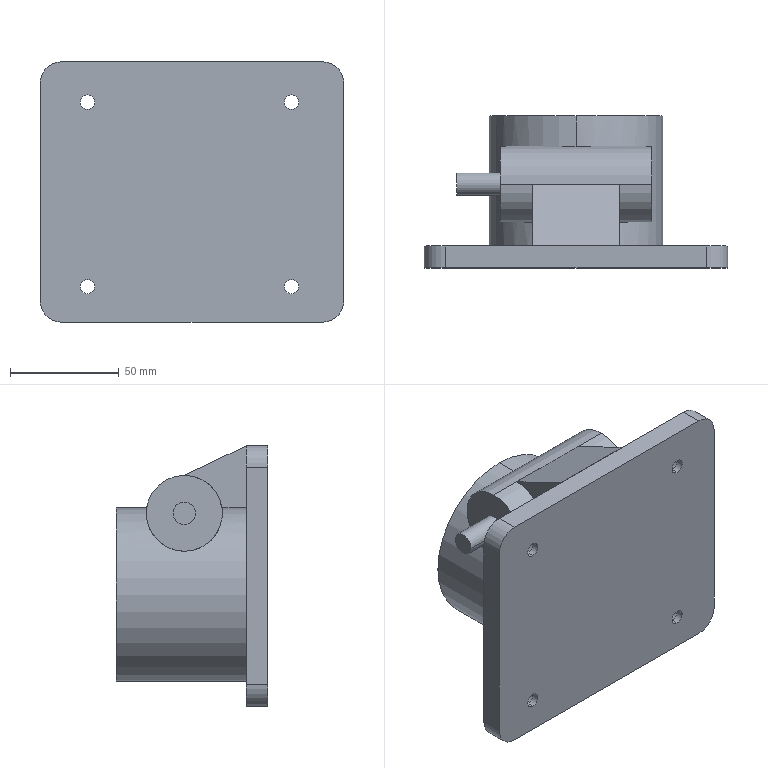Part | SolidWorks | features ICE 4, Extrusion 1, Fillet 1, HoleWzd 1 | 2 solids | 46 faces | box 140 x 70 x 120 mm | volume 525690 mm3 | cylinder 27 | plane 19 | commonest cylinder face diameters 6.6 x8 11 x8 20 x4 35 x3 10.271 x2 80 x2
STEP:
#1=CARTESIAN_POINT('',(-20.,11.222,40.));
#2=VERTEX_POINT('',#1);
#3=CARTESIAN_POINT('',(-20.,28.542,55.001));
#4=VERTEX_POINT('',#3);
#5=CARTESIAN_POINT('',(-20.,28.542,37.501));
#6=DIRECTION('',(-1.,0.,0.));
#7=DIRECTION('',(0.,0.,-1.));
#8=AXIS2_PLACEMENT_3D('',#5,#6,#7);
#9=CIRCLE('',#8,17.5);
#10=EDGE_CURVE('',#2,#4,#9,.T.);
#11=ORIENTED_EDGE('',*,*,#10,.T.);
#12=CARTESIAN_POINT('',(20.,28.542,55.001));
#13=VERTEX_POINT('',#12);
#14=CARTESIAN_POINT('',(20.,28.542,55.001));
#15=DIRECTION('',(-1.,0.,0.));
#16=VECTOR('',#15,1000.);
#17=LINE('',#14,#16);
#18=EDGE_CURVE('',#13,#4,#17,.T.);
#19=ORIENTED_EDGE('',*,*,#18,.F.);
#20=CARTESIAN_POINT('',(20.,11.222,40.));
#21=VERTEX_POINT('',#20);
#22=CARTESIAN_POINT('',(20.,28.542,37.501));
#23=DIRECTION('',(-1.,0.,0.));
#24=DIRECTION('',(0.,0.,-1.));
#25=AXIS2_PLACEMENT_3D('',#22,#23,#24);
#26=CIRCLE('',#25,17.5);
#27=EDGE_CURVE('',#21,#13,#26,.T.);
#28=ORIENTED_EDGE('',*,*,#27,.F.);
#29=CARTESIAN_POINT('',(20.,11.222,40.));
#30=DIRECTION('',(-1.,0.,0.));
#31=VECTOR('',#30,1000.);
#32=LINE('',#29,#31);
#33=EDGE_CURVE('',#21,#2,#32,.T.);
#34=ORIENTED_EDGE('',*,*,#33,.T.);
#35=EDGE_LOOP('',(#11,#19,#28,#34));
#36=FACE_OUTER_BOUND('',#35,.T.);
#37=CARTESIAN_POINT('',(20.,28.542,37.501));
#38=DIRECTION('',(-1.,0.,0.));
#39=DIRECTION('',(0.,0.,1.));
#40=AXIS2_PLACEMENT_3D('',#37,#38,#39);
#41=CYLINDRICAL_SURFACE('',#40,17.5);
#42=ADVANCED_FACE('',(#36),#41,.F.);
#43=CARTESIAN_POINT('',(-20.,0.,68.595));
#44=VERTEX_POINT('',#43);
#45=CARTESIAN_POINT('',(-20.,28.542,55.001));
#46=DIRECTION('',(0.,-0.9028,0.43));
#47=VECTOR('',#46,1000.);
#48=LINE('',#45,#47);
#49=EDGE_CURVE('',#4,#44,#48,.T.);
#50=ORIENTED_EDGE('',*,*,#49,.T.);
#51=CARTESIAN_POINT('',(20.,0.,68.595));
#52=VERTEX_POINT('',#51);
#53=CARTESIAN_POINT('',(20.,0.,68.595));
#54=DIRECTION('',(-1.,0.,0.));
#55=VECTOR('',#54,1000.);
#56=LINE('',#53,#55);
#57=EDGE_CURVE('',#52,#44,#56,.T.);
#58=ORIENTED_EDGE('',*,*,#57,.F.);
#59=CARTESIAN_POINT('',(20.,28.542,55.001));
#60=DIRECTION('',(0.,-0.9028,0.43));
#61=VECTOR('',#60,1000.);
#62=LINE('',#59,#61);
#63=EDGE_CURVE('',#13,#52,#62,.T.);
#64=ORIENTED_EDGE('',*,*,#63,.F.);
#65=ORIENTED_EDGE('',*,*,#18,.T.);
#66=EDGE_LOOP('',(#50,#58,#64,#65));
#67=FACE_OUTER_BOUND('',#66,.T.);
#68=CARTESIAN_POINT('',(20.,28.542,55.001));
#69=DIRECTION('',(0.,-0.43,-0.9028));
#70=DIRECTION('',(0.,0.9028,-0.43));
#71=AXIS2_PLACEMENT_3D('',#68,#69,#70);
#72=PLANE('',#71);
#73=ADVANCED_FACE('',(#67),#72,.F.);
#74=CARTESIAN_POINT('',(-20.,0.,40.));
#75=VERTEX_POINT('',#74);
#76=CARTESIAN_POINT('',(-20.,0.,68.595));
#77=DIRECTION('',(0.,0.,-1.));
#78=VECTOR('',#77,1000.);
#79=LINE('',#76,#78);
#80=EDGE_CURVE('',#44,#75,#79,.T.);
#81=ORIENTED_EDGE('',*,*,#80,.T.);
#82=CARTESIAN_POINT('',(20.,0.,40.));
#83=VERTEX_POINT('',#82);
#84=CARTESIAN_POINT('',(20.,0.,40.));
#85=DIRECTION('',(-1.,0.,0.));
#86=VECTOR('',#85,1000.);
#87=LINE('',#84,#86);
#88=EDGE_CURVE('',#83,#75,#87,.T.);
#89=ORIENTED_EDGE('',*,*,#88,.F.);
#90=CARTESIAN_POINT('',(20.,0.,68.595));
#91=DIRECTION('',(0.,0.,-1.));
#92=VECTOR('',#91,1000.);
#93=LINE('',#90,#92);
#94=EDGE_CURVE('',#52,#83,#93,.T.);
#95=ORIENTED_EDGE('',*,*,#94,.F.);
#96=ORIENTED_EDGE('',*,*,#57,.T.);
#97=EDGE_LOOP('',(#81,#89,#95,#96));
#98=FACE_OUTER_BOUND('',#97,.T.);
#99=CARTESIAN_POINT('',(20.,0.,68.595));
#100=DIRECTION('',(0.,1.,0.));
#101=DIRECTION('',(0.,0.,1.));
#102=AXIS2_PLACEMENT_3D('',#99,#100,#101);
#103=PLANE('',#102);
#104=ADVANCED_FACE('',(#98),#103,.F.);
#105=CARTESIAN_POINT('',(-20.,0.,40.));
#106=DIRECTION('',(0.,1.,0.));
#107=VECTOR('',#106,1000.);
#108=LINE('',#105,#107);
#109=EDGE_CURVE('',#75,#2,#108,.T.);
#110=ORIENTED_EDGE('',*,*,#109,.T.);
#111=ORIENTED_EDGE('',*,*,#33,.F.);
#112=CARTESIAN_POINT('',(20.,0.,40.));
#113=DIRECTION('',(0.,1.,0.));
#114=VECTOR('',#113,1000.);
#115=LINE('',#112,#114);
#116=EDGE_CURVE('',#83,#21,#115,.T.);
#117=ORIENTED_EDGE('',*,*,#116,.F.);
#118=ORIENTED_EDGE('',*,*,#88,.T.);
#119=EDGE_LOOP('',(#110,#111,#117,#118));
#120=FACE_OUTER_BOUND('',#119,.T.);
#121=CARTESIAN_POINT('',(20.,0.,40.));
#122=DIRECTION('',(0.,0.,1.));
#123=DIRECTION('',(1.,0.,0.));
#124=AXIS2_PLACEMENT_3D('',#121,#122,#123);
#125=PLANE('',#124);
#126=ADVANCED_FACE('',(#120),#125,.F.);
#127=ORIENTED_EDGE('',*,*,#27,.T.);
#128=ORIENTED_EDGE('',*,*,#63,.T.);
#129=ORIENTED_EDGE('',*,*,#94,.T.);
#130=ORIENTED_EDGE('',*,*,#116,.T.);
#131=EDGE_LOOP('',(#127,#128,#129,#130));
#132=FACE_OUTER_BOUND('',#131,.T.);
#133=CARTESIAN_POINT('',(20.,28.542,37.501));
#134=DIRECTION('',(1.,0.,0.));
#135=DIRECTION('',(0.,0.,-1.));
#136=AXIS2_PLACEMENT_3D('',#133,#134,#135);
#137=PLANE('',#136);
#138=ADVANCED_FACE('',(#132),#137,.T.);
#139=ORIENTED_EDGE('',*,*,#10,.F.);
#140=ORIENTED_EDGE('',*,*,#109,.F.);
#141=ORIENTED_EDGE('',*,*,#80,.F.);
#142=ORIENTED_EDGE('',*,*,#49,.F.);
#143=EDGE_LOOP('',(#139,#140,#141,#142));
#144=FACE_OUTER_BOUND('',#143,.T.);
#145=CARTESIAN_POINT('',(-20.,28.542,37.501));
#146=DIRECTION('',(1.,0.,0.));
#147=DIRECTION('',(0.,0.,-1.));
#148=AXIS2_PLACEMENT_3D('',#145,#146,#147);
#149=PLANE('',#148);
#150=ADVANCED_FACE('',(#144),#149,.F.);
#151=CLOSED_SHELL('',(#42,#73,#104,#126,#138,#150));
#152=MANIFOLD_SOLID_BREP('',#151);
#153=CARTESIAN_POINT('',(-55.,23.407,37.501));
#154=VERTEX_POINT('',#153);
#155=CARTESIAN_POINT('',(-55.,33.678,37.501));
#156=VERTEX_POINT('',#155);
#157=CARTESIAN_POINT('',(-55.,28.542,37.501));
#158=DIRECTION('',(-1.,0.,0.));
#159=DIRECTION('',(0.,-1.,0.));
#160=AXIS2_PLACEMENT_3D('',#157,#158,#159);
#161=CIRCLE('',#160,5.135);
#162=EDGE_CURVE('',#154,#156,#161,.T.);
#163=ORIENTED_EDGE('',*,*,#162,.F.);
#164=CARTESIAN_POINT('',(-35.,23.407,37.501));
#165=VERTEX_POINT('',#164);
#166=CARTESIAN_POINT('',(-55.,23.407,37.501));
#167=DIRECTION('',(1.,0.,0.));
#168=VECTOR('',#167,1000.);
#169=LINE('',#166,#168);
#170=EDGE_CURVE('',#154,#165,#169,.T.);
#171=ORIENTED_EDGE('',*,*,#170,.T.);
#172=CARTESIAN_POINT('',(-35.,33.678,37.501));
#173=VERTEX_POINT('',#172);
#174=CARTESIAN_POINT('',(-35.,28.542,37.501));
#175=DIRECTION('',(-1.,0.,0.));
#176=DIRECTION('',(0.,0.,-1.));
#177=AXIS2_PLACEMENT_3D('',#174,#175,#176);
#178=CIRCLE('',#177,5.135);
#179=EDGE_CURVE('',#165,#173,#178,.T.);
#180=ORIENTED_EDGE('',*,*,#179,.T.);
#181=CARTESIAN_POINT('',(-55.,33.678,37.501));
#182=DIRECTION('',(1.,0.,0.));
#183=VECTOR('',#182,1000.);
#184=LINE('',#181,#183);
#185=EDGE_CURVE('',#156,#173,#184,.T.);
#186=ORIENTED_EDGE('',*,*,#185,.F.);
#187=EDGE_LOOP('',(#163,#171,#180,#186));
#188=FACE_OUTER_BOUND('',#187,.T.);
#189=CARTESIAN_POINT('',(-55.,28.542,37.501));
#190=DIRECTION('',(1.,0.,0.));
#191=DIRECTION('',(0.,1.,0.));
#192=AXIS2_PLACEMENT_3D('',#189,#190,#191);
#193=CYLINDRICAL_SURFACE('',#192,5.135);
#194=ADVANCED_FACE('',(#188),#193,.T.);
#195=CARTESIAN_POINT('',(-48.166,-6.8,44.5));
#196=VERTEX_POINT('',#195);
#197=CARTESIAN_POINT('',(-48.166,-6.8,55.5));
#198=VERTEX_POINT('',#197);
#199=CARTESIAN_POINT('',(-48.166,-6.8,50.));
#200=DIRECTION('',(0.,1.,0.));
#201=DIRECTION('',(0.,0.,1.));
#202=AXIS2_PLACEMENT_3D('',#199,#200,#201);
#203=CIRCLE('',#202,5.5);
#204=EDGE_CURVE('',#196,#198,#203,.T.);
#205=ORIENTED_EDGE('',*,*,#204,.F.);
#206=CARTESIAN_POINT('',(-48.166,0.,44.5));
#207=VERTEX_POINT('',#206);
#208=CARTESIAN_POINT('',(-48.166,0.,44.5));
#209=DIRECTION('',(0.,1.,0.));
#210=VECTOR('',#209,1000.);
#211=LINE('',#208,#210);
#212=EDGE_CURVE('',#196,#207,#211,.T.);
#213=ORIENTED_EDGE('',*,*,#212,.T.);
#214=CARTESIAN_POINT('',(-48.166,0.,55.5));
#215=VERTEX_POINT('',#214);
#216=CARTESIAN_POINT('',(-48.166,0.,50.));
#217=DIRECTION('',(0.,1.,0.));
#218=DIRECTION('',(0.,0.,1.));
#219=AXIS2_PLACEMENT_3D('',#216,#217,#218);
#220=CIRCLE('',#219,5.5);
#221=EDGE_CURVE('',#207,#215,#220,.T.);
#222=ORIENTED_EDGE('',*,*,#221,.T.);
#223=CARTESIAN_POINT('',(-48.166,0.,55.5));
#224=DIRECTION('',(0.,1.,0.));
#225=VECTOR('',#224,1000.);
#226=LINE('',#223,#225);
#227=EDGE_CURVE('',#198,#215,#226,.T.);
#228=ORIENTED_EDGE('',*,*,#227,.F.);
#229=EDGE_LOOP('',(#205,#213,#222,#228));
#230=FACE_OUTER_BOUND('',#229,.T.);
#231=CARTESIAN_POINT('',(-48.166,0.,50.));
#232=DIRECTION('',(0.,1.,0.));
#233=DIRECTION('',(0.,0.,1.));
#234=AXIS2_PLACEMENT_3D('',#231,#232,#233);
#235=CYLINDRICAL_SURFACE('',#234,5.5);
#236=ADVANCED_FACE('',(#230),#235,.F.);
#237=CARTESIAN_POINT('',(-48.166,-10.,46.7));
#238=VERTEX_POINT('',#237);
#239=CARTESIAN_POINT('',(-48.166,-10.,53.3));
#240=VERTEX_POINT('',#239);
#241=CARTESIAN_POINT('',(-48.166,-10.,50.));
#242=DIRECTION('',(0.,1.,0.));
#243=DIRECTION('',(0.,0.,1.));
#244=AXIS2_PLACEMENT_3D('',#241,#242,#243);
#245=CIRCLE('',#244,3.3);
#246=EDGE_CURVE('',#238,#240,#245,.T.);
#247=ORIENTED_EDGE('',*,*,#246,.F.);
#248=CARTESIAN_POINT('',(-48.166,-6.8,46.7));
#249=VERTEX_POINT('',#248);
#250=CARTESIAN_POINT('',(-48.166,0.,46.7));
#251=DIRECTION('',(0.,1.,0.));
#252=VECTOR('',#251,1000.);
#253=LINE('',#250,#252);
#254=EDGE_CURVE('',#238,#249,#253,.T.);
#255=ORIENTED_EDGE('',*,*,#254,.T.);
#256=CARTESIAN_POINT('',(-48.166,-6.8,53.3));
#257=VERTEX_POINT('',#256);
#258=CARTESIAN_POINT('',(-48.166,-6.8,50.));
#259=DIRECTION('',(0.,1.,0.));
#260=DIRECTION('',(0.,0.,1.));
#261=AXIS2_PLACEMENT_3D('',#258,#259,#260);
#262=CIRCLE('',#261,3.3);
#263=EDGE_CURVE('',#249,#257,#262,.T.);
#264=ORIENTED_EDGE('',*,*,#263,.T.);
#265=CARTESIAN_POINT('',(-48.166,0.,53.3));
#266=DIRECTION('',(0.,1.,0.));
#267=VECTOR('',#266,1000.);
#268=LINE('',#265,#267);
#269=EDGE_CURVE('',#240,#257,#268,.T.);
#270=ORIENTED_EDGE('',*,*,#269,.F.);
#271=EDGE_LOOP('',(#247,#255,#264,#270));
#272=FACE_OUTER_BOUND('',#271,.T.);
#273=CARTESIAN_POINT('',(-48.166,0.,50.));
#274=DIRECTION('',(0.,1.,0.));
#275=DIRECTION('',(0.,0.,1.));
#276=AXIS2_PLACEMENT_3D('',#273,#274,#275);
#277=CYLINDRICAL_SURFACE('',#276,3.3);
#278=ADVANCED_FACE('',(#272),#277,.F.);
#279=CARTESIAN_POINT('',(-48.166,-6.8,-40.5));
#280=VERTEX_POINT('',#279);
#281=CARTESIAN_POINT('',(-48.166,-6.8,-29.5));
#282=VERTEX_POINT('',#281);
#283=CARTESIAN_POINT('',(-48.166,-6.8,-35.));
#284=DIRECTION('',(0.,1.,0.));
#285=DIRECTION('',(0.,0.,1.));
#286=AXIS2_PLACEMENT_3D('',#283,#284,#285);
#287=CIRCLE('',#286,5.5);
#288=EDGE_CURVE('',#280,#282,#287,.T.);
#289=ORIENTED_EDGE('',*,*,#288,.F.);
#290=CARTESIAN_POINT('',(-48.166,0.,-40.5));
#291=VERTEX_POINT('',#290);
#292=CARTESIAN_POINT('',(-48.166,0.,-40.5));
#293=DIRECTION('',(0.,1.,0.));
#294=VECTOR('',#293,1000.);
#295=LINE('',#292,#294);
#296=EDGE_CURVE('',#280,#291,#295,.T.);
#297=ORIENTED_EDGE('',*,*,#296,.T.);
#298=CARTESIAN_POINT('',(-48.166,0.,-29.5));
#299=VERTEX_POINT('',#298);
#300=CARTESIAN_POINT('',(-48.166,0.,-35.));
#301=DIRECTION('',(0.,1.,0.));
#302=DIRECTION('',(0.,0.,1.));
#303=AXIS2_PLACEMENT_3D('',#300,#301,#302);
#304=CIRCLE('',#303,5.5);
#305=EDGE_CURVE('',#291,#299,#304,.T.);
#306=ORIENTED_EDGE('',*,*,#305,.T.);
#307=CARTESIAN_POINT('',(-48.166,0.,-29.5));
#308=DIRECTION('',(0.,1.,0.));
#309=VECTOR('',#308,1000.);
#310=LINE('',#307,#309);
#311=EDGE_CURVE('',#282,#299,#310,.T.);
#312=ORIENTED_EDGE('',*,*,#311,.F.);
#313=EDGE_LOOP('',(#289,#297,#306,#312));
#314=FACE_OUTER_BOUND('',#313,.T.);
#315=CARTESIAN_POINT('',(-48.166,0.,-35.));
#316=DIRECTION('',(0.,1.,0.));
#317=DIRECTION('',(0.,0.,1.));
#318=AXIS2_PLACEMENT_3D('',#315,#316,#317);
#319=CYLINDRICAL_SURFACE('',#318,5.5);
#320=ADVANCED_FACE('',(#314),#319,.F.);
#321=CARTESIAN_POINT('',(-48.166,-10.,-38.3));
#322=VERTEX_POINT('',#321);
#323=CARTESIAN_POINT('',(-48.166,-10.,-31.7));
#324=VERTEX_POINT('',#323);
#325=CARTESIAN_POINT('',(-48.166,-10.,-35.));
#326=DIRECTION('',(0.,1.,0.));
#327=DIRECTION('',(0.,0.,1.));
#328=AXIS2_PLACEMENT_3D('',#325,#326,#327);
#329=CIRCLE('',#328,3.3);
#330=EDGE_CURVE('',#322,#324,#329,.T.);
#331=ORIENTED_EDGE('',*,*,#330,.F.);
#332=CARTESIAN_POINT('',(-48.166,-6.8,-38.3));
#333=VERTEX_POINT('',#332);
#334=CARTESIAN_POINT('',(-48.166,0.,-38.3));
#335=DIRECTION('',(0.,1.,0.));
#336=VECTOR('',#335,1000.);
#337=LINE('',#334,#336);
#338=EDGE_CURVE('',#322,#333,#337,.T.);
#339=ORIENTED_EDGE('',*,*,#338,.T.);
#340=CARTESIAN_POINT('',(-48.166,-6.8,-31.7));
#341=VERTEX_POINT('',#340);
#342=CARTESIAN_POINT('',(-48.166,-6.8,-35.));
#343=DIRECTION('',(0.,1.,0.));
#344=DIRECTION('',(0.,0.,1.));
#345=AXIS2_PLACEMENT_3D('',#342,#343,#344);
#346=CIRCLE('',#345,3.3);
#347=EDGE_CURVE('',#333,#341,#346,.T.);
#348=ORIENTED_EDGE('',*,*,#347,.T.);
#349=CARTESIAN_POINT('',(-48.166,0.,-31.7));
#350=DIRECTION('',(0.,1.,0.));
#351=VECTOR('',#350,1000.);
#352=LINE('',#349,#351);
#353=EDGE_CURVE('',#324,#341,#352,.T.);
#354=ORIENTED_EDGE('',*,*,#353,.F.);
#355=EDGE_LOOP('',(#331,#339,#348,#354));
#356=FACE_OUTER_BOUND('',#355,.T.);
#357=CARTESIAN_POINT('',(-48.166,0.,-35.));
#358=DIRECTION('',(0.,1.,0.));
#359=DIRECTION('',(0.,0.,1.));
#360=AXIS2_PLACEMENT_3D('',#357,#358,#359);
#361=CYLINDRICAL_SURFACE('',#360,3.3);
#362=ADVANCED_FACE('',(#356),#361,.F.);
#363=CARTESIAN_POINT('',(45.834,-6.8,-40.5));
#364=VERTEX_POINT('',#363);
#365=CARTESIAN_POINT('',(45.834,-6.8,-29.5));
#366=VERTEX_POINT('',#365);
#367=CARTESIAN_POINT('',(45.834,-6.8,-35.));
#368=DIRECTION('',(0.,1.,0.));
#369=DIRECTION('',(0.,0.,1.));
#370=AXIS2_PLACEMENT_3D('',#367,#368,#369);
#371=CIRCLE('',#370,5.5);
#372=EDGE_CURVE('',#364,#366,#371,.T.);
#373=ORIENTED_EDGE('',*,*,#372,.F.);
#374=CARTESIAN_POINT('',(45.834,0.,-40.5));
#375=VERTEX_POINT('',#374);
#376=CARTESIAN_POINT('',(45.834,0.,-40.5));
#377=DIRECTION('',(0.,1.,0.));
#378=VECTOR('',#377,1000.);
#379=LINE('',#376,#378);
#380=EDGE_CURVE('',#364,#375,#379,.T.);
#381=ORIENTED_EDGE('',*,*,#380,.T.);
#382=CARTESIAN_POINT('',(45.834,0.,-29.5));
#383=VERTEX_POINT('',#382);
#384=CARTESIAN_POINT('',(45.834,0.,-35.));
#385=DIRECTION('',(0.,1.,0.));
#386=DIRECTION('',(0.,0.,1.));
#387=AXIS2_PLACEMENT_3D('',#384,#385,#386);
#388=CIRCLE('',#387,5.5);
#389=EDGE_CURVE('',#375,#383,#388,.T.);
#390=ORIENTED_EDGE('',*,*,#389,.T.);
#391=CARTESIAN_POINT('',(45.834,0.,-29.5));
#392=DIRECTION('',(0.,1.,0.));
#393=VECTOR('',#392,1000.);
#394=LINE('',#391,#393);
#395=EDGE_CURVE('',#366,#383,#394,.T.);
#396=ORIENTED_EDGE('',*,*,#395,.F.);
#397=EDGE_LOOP('',(#373,#381,#390,#396));
#398=FACE_OUTER_BOUND('',#397,.T.);
#399=CARTESIAN_POINT('',(45.834,0.,-35.));
#400=DIRECTION('',(0.,1.,0.));
#401=DIRECTION('',(0.,0.,1.));
#402=AXIS2_PLACEMENT_3D('',#399,#400,#401);
#403=CYLINDRICAL_SURFACE('',#402,5.5);
#404=ADVANCED_FACE('',(#398),#403,.F.);
#405=CARTESIAN_POINT('',(45.834,-10.,-38.3));
#406=VERTEX_POINT('',#405);
#407=CARTESIAN_POINT('',(45.834,-10.,-31.7));
#408=VERTEX_POINT('',#407);
#409=CARTESIAN_POINT('',(45.834,-10.,-35.));
#410=DIRECTION('',(0.,1.,0.));
#411=DIRECTION('',(0.,0.,1.));
#412=AXIS2_PLACEMENT_3D('',#409,#410,#411);
#413=CIRCLE('',#412,3.3);
#414=EDGE_CURVE('',#406,#408,#413,.T.);
#415=ORIENTED_EDGE('',*,*,#414,.F.);
#416=CARTESIAN_POINT('',(45.834,-6.8,-38.3));
#417=VERTEX_POINT('',#416);
#418=CARTESIAN_POINT('',(45.834,0.,-38.3));
#419=DIRECTION('',(0.,1.,0.));
#420=VECTOR('',#419,1000.);
#421=LINE('',#418,#420);
#422=EDGE_CURVE('',#406,#417,#421,.T.);
#423=ORIENTED_EDGE('',*,*,#422,.T.);
#424=CARTESIAN_POINT('',(45.834,-6.8,-31.7));
#425=VERTEX_POINT('',#424);
#426=CARTESIAN_POINT('',(45.834,-6.8,-35.));
#427=DIRECTION('',(0.,1.,0.));
#428=DIRECTION('',(0.,0.,1.));
#429=AXIS2_PLACEMENT_3D('',#426,#427,#428);
#430=CIRCLE('',#429,3.3);
#431=EDGE_CURVE('',#417,#425,#430,.T.);
#432=ORIENTED_EDGE('',*,*,#431,.T.);
#433=CARTESIAN_POINT('',(45.834,0.,-31.7));
#434=DIRECTION('',(0.,1.,0.));
#435=VECTOR('',#434,1000.);
#436=LINE('',#433,#435);
#437=EDGE_CURVE('',#408,#425,#436,.T.);
#438=ORIENTED_EDGE('',*,*,#437,.F.);
#439=EDGE_LOOP('',(#415,#423,#432,#438));
#440=FACE_OUTER_BOUND('',#439,.T.);
#441=CARTESIAN_POINT('',(45.834,0.,-35.));
#442=DIRECTION('',(0.,1.,0.));
#443=DIRECTION('',(0.,0.,1.));
#444=AXIS2_PLACEMENT_3D('',#441,#442,#443);
#445=CYLINDRICAL_SURFACE('',#444,3.3);
#446=ADVANCED_FACE('',(#440),#445,.F.);
#447=CARTESIAN_POINT('',(45.834,-6.8,44.5));
#448=VERTEX_POINT('',#447);
#449=CARTESIAN_POINT('',(45.834,-6.8,55.5));
#450=VERTEX_POINT('',#449);
#451=CARTESIAN_POINT('',(45.834,-6.8,50.));
#452=DIRECTION('',(0.,1.,0.));
#453=DIRECTION('',(0.,0.,1.));
#454=AXIS2_PLACEMENT_3D('',#451,#452,#453);
#455=CIRCLE('',#454,5.5);
#456=EDGE_CURVE('',#448,#450,#455,.T.);
#457=ORIENTED_EDGE('',*,*,#456,.F.);
#458=CARTESIAN_POINT('',(45.834,0.,44.5));
#459=VERTEX_POINT('',#458);
#460=CARTESIAN_POINT('',(45.834,0.,44.5));
#461=DIRECTION('',(0.,1.,0.));
#462=VECTOR('',#461,1000.);
#463=LINE('',#460,#462);
#464=EDGE_CURVE('',#448,#459,#463,.T.);
#465=ORIENTED_EDGE('',*,*,#464,.T.);
#466=CARTESIAN_POINT('',(45.834,0.,55.5));
#467=VERTEX_POINT('',#466);
#468=CARTESIAN_POINT('',(45.834,0.,50.));
#469=DIRECTION('',(0.,1.,0.));
#470=DIRECTION('',(0.,0.,1.));
#471=AXIS2_PLACEMENT_3D('',#468,#469,#470);
#472=CIRCLE('',#471,5.5);
#473=EDGE_CURVE('',#459,#467,#472,.T.);
#474=ORIENTED_EDGE('',*,*,#473,.T.);
#475=CARTESIAN_POINT('',(45.834,0.,55.5));
#476=DIRECTION('',(0.,1.,0.));
#477=VECTOR('',#476,1000.);
#478=LINE('',#475,#477);
#479=EDGE_CURVE('',#450,#467,#478,.T.);
#480=ORIENTED_EDGE('',*,*,#479,.F.);
#481=EDGE_LOOP('',(#457,#465,#474,#480));
#482=FACE_OUTER_BOUND('',#481,.T.);
#483=CARTESIAN_POINT('',(45.834,0.,50.));
#484=DIRECTION('',(0.,1.,0.));
#485=DIRECTION('',(0.,0.,1.));
#486=AXIS2_PLACEMENT_3D('',#483,#484,#485);
#487=CYLINDRICAL_SURFACE('',#486,5.5);
#488=ADVANCED_FACE('',(#482),#487,.F.);
#489=CARTESIAN_POINT('',(45.834,-10.,46.7));
#490=VERTEX_POINT('',#489);
#491=CARTESIAN_POINT('',(45.834,-10.,53.3));
#492=VERTEX_POINT('',#491);
#493=CARTESIAN_POINT('',(45.834,-10.,50.));
#494=DIRECTION('',(0.,1.,0.));
#495=DIRECTION('',(0.,0.,1.));
#496=AXIS2_PLACEMENT_3D('',#493,#494,#495);
#497=CIRCLE('',#496,3.3);
#498=EDGE_CURVE('',#490,#492,#497,.T.);
#499=ORIENTED_EDGE('',*,*,#498,.F.);
#500=CARTESIAN_POINT('',(45.834,-6.8,46.7));
#501=VERTEX_POINT('',#500);
#502=CARTESIAN_POINT('',(45.834,0.,46.7));
#503=DIRECTION('',(0.,1.,0.));
#504=VECTOR('',#503,1000.);
#505=LINE('',#502,#504);
#506=EDGE_CURVE('',#490,#501,#505,.T.);
#507=ORIENTED_EDGE('',*,*,#506,.T.);
#508=CARTESIAN_POINT('',(45.834,-6.8,53.3));
#509=VERTEX_POINT('',#508);
#510=CARTESIAN_POINT('',(45.834,-6.8,50.));
#511=DIRECTION('',(0.,1.,0.));
#512=DIRECTION('',(0.,0.,1.));
#513=AXIS2_PLACEMENT_3D('',#510,#511,#512);
#514=CIRCLE('',#513,3.3);
#515=EDGE_CURVE('',#501,#509,#514,.T.);
#516=ORIENTED_EDGE('',*,*,#515,.T.);
#517=CARTESIAN_POINT('',(45.834,0.,53.3));
#518=DIRECTION('',(0.,1.,0.));
#519=VECTOR('',#518,1000.);
#520=LINE('',#517,#519);
#521=EDGE_CURVE('',#492,#509,#520,.T.);
#522=ORIENTED_EDGE('',*,*,#521,.F.);
#523=EDGE_LOOP('',(#499,#507,#516,#522));
#524=FACE_OUTER_BOUND('',#523,.T.);
#525=CARTESIAN_POINT('',(45.834,0.,50.));
#526=DIRECTION('',(0.,1.,0.));
#527=DIRECTION('',(0.,0.,1.));
#528=AXIS2_PLACEMENT_3D('',#525,#526,#527);
#529=CYLINDRICAL_SURFACE('',#528,3.3);
#530=ADVANCED_FACE('',(#524),#529,.F.);
#531=CARTESIAN_POINT('',(35.,28.542,20.001));
#532=VERTEX_POINT('',#531);
#533=CARTESIAN_POINT('',(35.,28.542,55.001));
#534=VERTEX_POINT('',#533);
#535=CARTESIAN_POINT('',(35.,28.542,37.501));
#536=DIRECTION('',(1.,0.,0.));
#537=DIRECTION('',(0.,0.,-1.));
#538=AXIS2_PLACEMENT_3D('',#535,#536,#537);
#539=CIRCLE('',#538,17.5);
#540=EDGE_CURVE('',#532,#534,#539,.T.);
#541=ORIENTED_EDGE('',*,*,#540,.F.);
#542=CARTESIAN_POINT('',(34.64,28.542,20.001));
#543=VERTEX_POINT('',#542);
#544=CARTESIAN_POINT('',(35.,28.542,20.001));
#545=DIRECTION('',(-1.,0.,0.));
#546=VECTOR('',#545,1000.);
#547=LINE('',#544,#546);
#548=EDGE_CURVE('',#532,#543,#547,.T.);
#549=ORIENTED_EDGE('',*,*,#548,.T.);
#550=CARTESIAN_POINT('',(0.,45.863,40.));
#551=VERTEX_POINT('',#550);
#552=CARTESIAN_POINT('',(34.64,28.542,20.001));
#553=CARTESIAN_POINT('',(34.64,29.605,20.001));
#554=CARTESIAN_POINT('',(34.586,30.662,20.097));
#555=CARTESIAN_POINT('',(34.414,32.239,20.388));
#556=CARTESIAN_POINT('',(34.343,32.756,20.508));
#557=CARTESIAN_POINT('',(34.172,33.768,20.791));
#558=CARTESIAN_POINT('',(34.073,34.263,20.954));
#559=CARTESIAN_POINT('',(33.844,35.233,21.322));
#560=CARTESIAN_POINT('',(33.714,35.707,21.527));
#561=CARTESIAN_POINT('',(33.423,36.636,21.976));
#562=CARTESIAN_POINT('',(33.261,37.088,22.221));
#563=CARTESIAN_POINT('',(32.735,38.385,22.996));
#564=CARTESIAN_POINT('',(32.326,39.179,23.571));
#565=CARTESIAN_POINT('',(31.617,40.272,24.505));
#566=CARTESIAN_POINT('',(31.364,40.621,24.829));
#567=CARTESIAN_POINT('',(30.832,41.275,25.487));
#568=CARTESIAN_POINT('',(30.553,41.582,25.821));
#569=CARTESIAN_POINT('',(29.968,42.157,26.497));
#570=CARTESIAN_POINT('',(29.662,42.426,26.84));
#571=CARTESIAN_POINT('',(29.024,42.929,27.529));
#572=CARTESIAN_POINT('',(28.69,43.164,27.877));
#573=CARTESIAN_POINT('',(27.652,43.816,28.919));
#574=CARTESIAN_POINT('',(26.922,44.175,29.602));
#575=CARTESIAN_POINT('',(25.386,44.778,30.928));
#576=CARTESIAN_POINT('',(24.581,45.021,31.573));
#577=CARTESIAN_POINT('',(23.318,45.317,32.505));
#578=CARTESIAN_POINT('',(22.887,45.405,32.81));
#579=CARTESIAN_POINT('',(22.011,45.559,33.403));
#580=CARTESIAN_POINT('',(21.568,45.625,33.691));
#581=CARTESIAN_POINT('',(20.224,45.797,34.527));
#582=CARTESIAN_POINT('',(19.308,45.876,35.047));
#583=CARTESIAN_POINT('',(17.435,45.986,36.016));
#584=CARTESIAN_POINT('',(16.479,46.016,36.463));
#585=CARTESIAN_POINT('',(14.527,46.046,37.284));
#586=CARTESIAN_POINT('',(13.529,46.045,37.658));
#587=CARTESIAN_POINT('',(10.491,46.017,38.659));
#588=CARTESIAN_POINT('',(8.434,45.967,39.158));
#589=CARTESIAN_POINT('',(5.304,45.909,39.661));
#590=CARTESIAN_POINT('',(4.254,45.893,39.787));
#591=CARTESIAN_POINT('',(2.136,45.869,39.957));
#592=CARTESIAN_POINT('',(1.067,45.863,40.));
#593=CARTESIAN_POINT('',(0.,45.863,40.));
#594=B_SPLINE_CURVE_WITH_KNOTS('',3,(#552,#553,#554,#555,#556,#557,#558,#559,#560,#561,#562,#563,#564,#565,#566,#567,#568,#569,#570,#571,#572,#573,#574,#575,#576,#577,#578,#579,#580,#581,#582,#583,#584,#585,#586,#587,#588,#589,#590,#591,#592,#593),.UNSPECIFIED.,.F.,.F.,(4,2,2,2,2,2,2,2,2,2,2,2,2,2,2,2,2,2,2,2,4),(0.1517,0.1549,0.1564,0.158,0.1596,0.1612,0.1643,0.1659,0.1675,0.1691,0.1706,0.1738,0.177,0.1785,0.1801,0.1833,0.1864,0.1896,0.1959,0.199,0.2022),.UNSPECIFIED.);
#595=EDGE_CURVE('',#543,#551,#594,.T.);
#596=ORIENTED_EDGE('',*,*,#595,.T.);
#597=CARTESIAN_POINT('',(-34.64,28.542,20.001));
#598=VERTEX_POINT('',#597);
#599=CARTESIAN_POINT('',(0.,45.863,40.));
#600=CARTESIAN_POINT('',(-2.138,45.863,40.));
#601=CARTESIAN_POINT('',(-4.248,45.89,39.83));
#602=CARTESIAN_POINT('',(-8.411,45.967,39.163));
#603=CARTESIAN_POINT('',(-10.464,46.016,38.666));
#604=CARTESIAN_POINT('',(-12.996,46.04,37.834));
#605=CARTESIAN_POINT('',(-13.501,46.043,37.656));
#606=CARTESIAN_POINT('',(-14.5,46.042,37.283));
#607=CARTESIAN_POINT('',(-14.994,46.039,37.087));
#608=CARTESIAN_POINT('',(-16.461,46.017,36.471));
#609=CARTESIAN_POINT('',(-17.419,45.987,36.023));
#610=CARTESIAN_POINT('',(-19.295,45.877,35.055));
#611=CARTESIAN_POINT('',(-20.212,45.798,34.534));
#612=CARTESIAN_POINT('',(-21.557,45.627,33.699));
#613=CARTESIAN_POINT('',(-22.,45.56,33.411));
#614=CARTESIAN_POINT('',(-22.875,45.407,32.818));
#615=CARTESIAN_POINT('',(-23.308,45.319,32.512));
#616=CARTESIAN_POINT('',(-24.575,45.023,31.578));
#617=CARTESIAN_POINT('',(-25.382,44.779,30.932));
#618=CARTESIAN_POINT('',(-26.921,44.175,29.602));
#619=CARTESIAN_POINT('',(-27.653,43.815,28.919));
#620=CARTESIAN_POINT('',(-29.039,42.945,27.526));
#621=CARTESIAN_POINT('',(-29.677,42.444,26.834));
#622=CARTESIAN_POINT('',(-30.553,41.582,25.821));
#623=CARTESIAN_POINT('',(-30.831,41.276,25.487));
#624=CARTESIAN_POINT('',(-31.362,40.624,24.832));
#625=CARTESIAN_POINT('',(-31.615,40.276,24.508));
#626=CARTESIAN_POINT('',(-32.328,39.177,23.57));
#627=CARTESIAN_POINT('',(-32.735,38.383,22.996));
#628=CARTESIAN_POINT('',(-33.258,37.097,22.226));
#629=CARTESIAN_POINT('',(-33.417,36.652,21.985));
#630=CARTESIAN_POINT('',(-33.708,35.729,21.537));
#631=CARTESIAN_POINT('',(-33.84,35.247,21.328));
#632=CARTESIAN_POINT('',(-34.187,33.78,20.77));
#633=CARTESIAN_POINT('',(-34.356,32.77,20.487));
#634=CARTESIAN_POINT('',(-34.526,31.21,20.197));
#635=CARTESIAN_POINT('',(-34.569,30.682,20.124));
#636=CARTESIAN_POINT('',(-34.626,29.609,20.025));
#637=CARTESIAN_POINT('',(-34.64,29.075,20.001));
#638=CARTESIAN_POINT('',(-34.64,28.542,20.001));
#639=B_SPLINE_CURVE_WITH_KNOTS('',3,(#599,#600,#601,#602,#603,#604,#605,#606,#607,#608,#609,#610,#611,#612,#613,#614,#615,#616,#617,#618,#619,#620,#621,#622,#623,#624,#625,#626,#627,#628,#629,#630,#631,#632,#633,#634,#635,#636,#637,#638),.UNSPECIFIED.,.F.,.F.,(4,2,2,2,2,2,2,2,2,2,2,2,2,2,2,2,2,2,2,4),(0.,0.006325,0.01265,0.01423,0.01581,0.01897,0.02214,0.02372,0.0253,0.02846,0.03162,0.03479,0.03637,0.03795,0.04111,0.04269,0.04427,0.04743,0.04902,0.0506),.UNSPECIFIED.);
#640=EDGE_CURVE('',#551,#598,#639,.T.);
#641=ORIENTED_EDGE('',*,*,#640,.T.);
#642=CARTESIAN_POINT('',(-35.,28.542,20.001));
#643=VERTEX_POINT('',#642);
#644=CARTESIAN_POINT('',(35.,28.542,20.001));
#645=DIRECTION('',(-1.,0.,0.));
#646=VECTOR('',#645,1000.);
#647=LINE('',#644,#646);
#648=EDGE_CURVE('',#598,#643,#647,.T.);
#649=ORIENTED_EDGE('',*,*,#648,.T.);
#650=CARTESIAN_POINT('',(-35.,28.542,55.001));
#651=VERTEX_POINT('',#650);
#652=CARTESIAN_POINT('',(-35.,28.542,37.501));
#653=DIRECTION('',(1.,0.,0.));
#654=DIRECTION('',(0.,0.,-1.));
#655=AXIS2_PLACEMENT_3D('',#652,#653,#654);
#656=CIRCLE('',#655,17.5);
#657=EDGE_CURVE('',#643,#651,#656,.T.);
#658=ORIENTED_EDGE('',*,*,#657,.T.);
#659=CARTESIAN_POINT('',(35.,28.542,55.001));
#660=DIRECTION('',(-1.,0.,0.));
#661=VECTOR('',#660,1000.);
#662=LINE('',#659,#661);
#663=EDGE_CURVE('',#534,#651,#662,.T.);
#664=ORIENTED_EDGE('',*,*,#663,.F.);
#665=EDGE_LOOP('',(#541,#549,#596,#641,#649,#658,#664));
#666=FACE_OUTER_BOUND('',#665,.T.);
#667=CARTESIAN_POINT('',(35.,28.542,37.501));
#668=DIRECTION('',(-1.,0.,0.));
#669=DIRECTION('',(0.,0.,1.));
#670=AXIS2_PLACEMENT_3D('',#667,#668,#669);
#671=CYLINDRICAL_SURFACE('',#670,17.5);
#672=ADVANCED_FACE('',(#666),#671,.T.);
#673=CARTESIAN_POINT('',(0.,60.,40.));
#674=VERTEX_POINT('',#673);
#675=CARTESIAN_POINT('',(0.,60.,-40.));
#676=VERTEX_POINT('',#675);
#677=CARTESIAN_POINT('',(0.,60.,0.));
#678=DIRECTION('',(0.,1.,0.));
#679=DIRECTION('',(0.,0.,1.));
#680=AXIS2_PLACEMENT_3D('',#677,#678,#679);
#681=CIRCLE('',#680,40.);
#682=EDGE_CURVE('',#674,#676,#681,.T.);
#683=ORIENTED_EDGE('',*,*,#682,.F.);
#684=CARTESIAN_POINT('',(0.,60.,40.));
#685=DIRECTION('',(0.,-1.,0.));
#686=VECTOR('',#685,1000.);
#687=LINE('',#684,#686);
#688=EDGE_CURVE('',#674,#551,#687,.T.);
#689=ORIENTED_EDGE('',*,*,#688,.T.);
#690=ORIENTED_EDGE('',*,*,#595,.F.);
#691=CARTESIAN_POINT('',(0.,11.222,40.));
#692=VERTEX_POINT('',#691);
#693=CARTESIAN_POINT('',(0.,11.222,40.));
#694=CARTESIAN_POINT('',(2.132,11.222,40.));
#695=CARTESIAN_POINT('',(4.238,11.195,39.831));
#696=CARTESIAN_POINT('',(8.401,11.118,39.165));
#697=CARTESIAN_POINT('',(10.459,11.069,38.668));
#698=CARTESIAN_POINT('',(14.522,11.03,37.332));
#699=CARTESIAN_POINT('',(16.475,11.043,36.511));
#700=CARTESIAN_POINT('',(19.289,11.207,35.058));
#701=CARTESIAN_POINT('',(20.207,11.286,34.537));
#702=CARTESIAN_POINT('',(22.003,11.515,33.421));
#703=CARTESIAN_POINT('',(22.885,11.667,32.823));
#704=CARTESIAN_POINT('',(24.572,12.061,31.58));
#705=CARTESIAN_POINT('',(25.379,12.305,30.935));
#706=CARTESIAN_POINT('',(26.534,12.757,29.937));
#707=CARTESIAN_POINT('',(26.91,12.923,29.599));
#708=CARTESIAN_POINT('',(27.643,13.288,28.916));
#709=CARTESIAN_POINT('',(28.001,13.488,28.569));
#710=CARTESIAN_POINT('',(29.039,14.14,27.526));
#711=CARTESIAN_POINT('',(29.676,14.64,26.836));
#712=CARTESIAN_POINT('',(30.552,15.502,25.822));
#713=CARTESIAN_POINT('',(30.83,15.808,25.489));
#714=CARTESIAN_POINT('',(31.362,16.461,24.832));
#715=CARTESIAN_POINT('',(31.616,16.811,24.507));
#716=CARTESIAN_POINT('',(32.327,17.906,23.571));
#717=CARTESIAN_POINT('',(32.734,18.699,22.998));
#718=CARTESIAN_POINT('',(33.257,19.986,22.227));
#719=CARTESIAN_POINT('',(33.417,20.431,21.986));
#720=CARTESIAN_POINT('',(33.709,21.357,21.536));
#721=CARTESIAN_POINT('',(33.841,21.839,21.328));
#722=CARTESIAN_POINT('',(34.187,23.303,20.771));
#723=CARTESIAN_POINT('',(34.356,24.312,20.487));
#724=CARTESIAN_POINT('',(34.526,25.875,20.197));
#725=CARTESIAN_POINT('',(34.569,26.407,20.124));
#726=CARTESIAN_POINT('',(34.626,27.477,20.025));
#727=CARTESIAN_POINT('',(34.64,28.01,20.001));
#728=CARTESIAN_POINT('',(34.64,28.542,20.001));
#729=B_SPLINE_CURVE_WITH_KNOTS('',3,(#693,#694,#695,#696,#697,#698,#699,#700,#701,#702,#703,#704,#705,#706,#707,#708,#709,#710,#711,#712,#713,#714,#715,#716,#717,#718,#719,#720,#721,#722,#723,#724,#725,#726,#727,#728),.UNSPECIFIED.,.F.,.F.,(4,2,2,2,2,2,2,2,2,2,2,2,2,2,2,2,2,4),(0.1011,0.1074,0.1138,0.1201,0.1233,0.1264,0.1296,0.1312,0.1327,0.1359,0.1375,0.1391,0.1422,0.1438,0.1454,0.1485,0.1501,0.1517),.UNSPECIFIED.);
#730=EDGE_CURVE('',#692,#543,#729,.T.);
#731=ORIENTED_EDGE('',*,*,#730,.F.);
#732=CARTESIAN_POINT('',(0.,0.,40.));
#733=VERTEX_POINT('',#732);
#734=CARTESIAN_POINT('',(0.,60.,40.));
#735=DIRECTION('',(0.,-1.,0.));
#736=VECTOR('',#735,1000.);
#737=LINE('',#734,#736);
#738=EDGE_CURVE('',#692,#733,#737,.T.);
#739=ORIENTED_EDGE('',*,*,#738,.T.);
#740=CARTESIAN_POINT('',(0.,0.,-40.));
#741=VERTEX_POINT('',#740);
#742=CARTESIAN_POINT('',(0.,0.,0.));
#743=DIRECTION('',(0.,1.,0.));
#744=DIRECTION('',(0.,0.,1.));
#745=AXIS2_PLACEMENT_3D('',#742,#743,#744);
#746=CIRCLE('',#745,40.);
#747=EDGE_CURVE('',#733,#741,#746,.T.);
#748=ORIENTED_EDGE('',*,*,#747,.T.);
#749=CARTESIAN_POINT('',(0.,60.,-40.));
#750=DIRECTION('',(0.,-1.,0.));
#751=VECTOR('',#750,1000.);
#752=LINE('',#749,#751);
#753=EDGE_CURVE('',#676,#741,#752,.T.);
#754=ORIENTED_EDGE('',*,*,#753,.F.);
#755=EDGE_LOOP('',(#683,#689,#690,#731,#739,#748,#754));
#756=FACE_OUTER_BOUND('',#755,.T.);
#757=CARTESIAN_POINT('',(0.,60.,0.));
#758=DIRECTION('',(0.,-1.,0.));
#759=DIRECTION('',(0.,0.,-1.));
#760=AXIS2_PLACEMENT_3D('',#757,#758,#759);
#761=CYLINDRICAL_SURFACE('',#760,40.);
#762=ADVANCED_FACE('',(#756),#761,.T.);
#763=CARTESIAN_POINT('',(-48.166,-10.,50.));
#764=DIRECTION('',(0.,1.,0.));
#765=DIRECTION('',(0.,0.,1.));
#766=AXIS2_PLACEMENT_3D('',#763,#764,#765);
#767=CIRCLE('',#766,3.3);
#768=EDGE_CURVE('',#240,#238,#767,.T.);
#769=ORIENTED_EDGE('',*,*,#768,.T.);
#770=ORIENTED_EDGE('',*,*,#246,.T.);
#771=EDGE_LOOP('',(#769,#770));
#772=FACE_BOUND('',#771,.T.);
#773=CARTESIAN_POINT('',(-48.166,-10.,-35.));
#774=DIRECTION('',(0.,1.,0.));
#775=DIRECTION('',(0.,0.,1.));
#776=AXIS2_PLACEMENT_3D('',#773,#774,#775);
#777=CIRCLE('',#776,3.3);
#778=EDGE_CURVE('',#324,#322,#777,.T.);
#779=ORIENTED_EDGE('',*,*,#778,.T.);
#780=ORIENTED_EDGE('',*,*,#330,.T.);
#781=EDGE_LOOP('',(#779,#780));
#782=FACE_BOUND('',#781,.T.);
#783=CARTESIAN_POINT('',(45.834,-10.,-35.));
#784=DIRECTION('',(0.,1.,0.));
#785=DIRECTION('',(0.,0.,1.));
#786=AXIS2_PLACEMENT_3D('',#783,#784,#785);
#787=CIRCLE('',#786,3.3);
#788=EDGE_CURVE('',#408,#406,#787,.T.);
#789=ORIENTED_EDGE('',*,*,#788,.T.);
#790=ORIENTED_EDGE('',*,*,#414,.T.);
#791=EDGE_LOOP('',(#789,#790));
#792=FACE_BOUND('',#791,.T.);
#793=CARTESIAN_POINT('',(-70.,-10.,58.595));
#794=VERTEX_POINT('',#793);
#795=CARTESIAN_POINT('',(-70.,-10.,-41.405));
#796=VERTEX_POINT('',#795);
#797=CARTESIAN_POINT('',(-70.,-10.,68.595));
#798=DIRECTION('',(0.,0.,-1.));
#799=VECTOR('',#798,1000.);
#800=LINE('',#797,#799);
#801=EDGE_CURVE('',#794,#796,#800,.T.);
#802=ORIENTED_EDGE('',*,*,#801,.T.);
#803=CARTESIAN_POINT('',(-60.,-10.,-51.405));
#804=VERTEX_POINT('',#803);
#805=CARTESIAN_POINT('',(-60.,-10.,-41.405));
#806=DIRECTION('',(0.,-1.,0.));
#807=DIRECTION('',(0.,0.,-1.));
#808=AXIS2_PLACEMENT_3D('',#805,#806,#807);
#809=CIRCLE('',#808,10.);
#810=EDGE_CURVE('',#796,#804,#809,.T.);
#811=ORIENTED_EDGE('',*,*,#810,.T.);
#812=CARTESIAN_POINT('',(60.,-10.,-51.405));
#813=VERTEX_POINT('',#812);
#814=CARTESIAN_POINT('',(-70.,-10.,-51.405));
#815=DIRECTION('',(1.,0.,0.));
#816=VECTOR('',#815,1000.);
#817=LINE('',#814,#816);
#818=EDGE_CURVE('',#804,#813,#817,.T.);
#819=ORIENTED_EDGE('',*,*,#818,.T.);
#820=CARTESIAN_POINT('',(70.,-10.,-41.405));
#821=VERTEX_POINT('',#820);
#822=CARTESIAN_POINT('',(60.,-10.,-41.405));
#823=DIRECTION('',(0.,-1.,0.));
#824=DIRECTION('',(0.,0.,-1.));
#825=AXIS2_PLACEMENT_3D('',#822,#823,#824);
#826=CIRCLE('',#825,10.);
#827=EDGE_CURVE('',#813,#821,#826,.T.);
#828=ORIENTED_EDGE('',*,*,#827,.T.);
#829=CARTESIAN_POINT('',(70.,-10.,58.595));
#830=VERTEX_POINT('',#829);
#831=CARTESIAN_POINT('',(70.,-10.,68.595));
#832=DIRECTION('',(0.,0.,1.));
#833=VECTOR('',#832,1000.);
#834=LINE('',#831,#833);
#835=EDGE_CURVE('',#821,#830,#834,.T.);
#836=ORIENTED_EDGE('',*,*,#835,.T.);
#837=CARTESIAN_POINT('',(60.,-10.,68.595));
#838=VERTEX_POINT('',#837);
#839=CARTESIAN_POINT('',(60.,-10.,58.595));
#840=DIRECTION('',(0.,-1.,0.));
#841=DIRECTION('',(0.,0.,-1.));
#842=AXIS2_PLACEMENT_3D('',#839,#840,#841);
#843=CIRCLE('',#842,10.);
#844=EDGE_CURVE('',#830,#838,#843,.T.);
#845=ORIENTED_EDGE('',*,*,#844,.T.);
#846=CARTESIAN_POINT('',(-60.,-10.,68.595));
#847=VERTEX_POINT('',#846);
#848=CARTESIAN_POINT('',(-70.,-10.,68.595));
#849=DIRECTION('',(-1.,0.,0.));
#850=VECTOR('',#849,1000.);
#851=LINE('',#848,#850);
#852=EDGE_CURVE('',#838,#847,#851,.T.);
#853=ORIENTED_EDGE('',*,*,#852,.T.);
#854=CARTESIAN_POINT('',(-60.,-10.,58.595));
#855=DIRECTION('',(0.,-1.,0.));
#856=DIRECTION('',(0.,0.,-1.));
#857=AXIS2_PLACEMENT_3D('',#854,#855,#856);
#858=CIRCLE('',#857,10.);
#859=EDGE_CURVE('',#847,#794,#858,.T.);
#860=ORIENTED_EDGE('',*,*,#859,.T.);
#861=EDGE_LOOP('',(#802,#811,#819,#828,#836,#845,#853,#860));
#862=FACE_OUTER_BOUND('',#861,.T.);
#863=CARTESIAN_POINT('',(45.834,-10.,50.));
#864=DIRECTION('',(0.,1.,0.));
#865=DIRECTION('',(0.,0.,1.));
#866=AXIS2_PLACEMENT_3D('',#863,#864,#865);
#867=CIRCLE('',#866,3.3);
#868=EDGE_CURVE('',#492,#490,#867,.T.);
#869=ORIENTED_EDGE('',*,*,#868,.T.);
#870=ORIENTED_EDGE('',*,*,#498,.T.);
#871=EDGE_LOOP('',(#869,#870));
#872=FACE_BOUND('',#871,.T.);
#873=CARTESIAN_POINT('',(0.,-10.,0.));
#874=DIRECTION('',(0.,-1.,0.));
#875=DIRECTION('',(0.,0.,-1.));
#876=AXIS2_PLACEMENT_3D('',#873,#874,#875);
#877=PLANE('',#876);
#878=ADVANCED_FACE('',(#772,#782,#792,#862,#872),#877,.T.);
#879=CARTESIAN_POINT('',(-48.166,0.,50.));
#880=DIRECTION('',(0.,1.,0.));
#881=DIRECTION('',(0.,0.,1.));
#882=AXIS2_PLACEMENT_3D('',#879,#880,#881);
#883=CIRCLE('',#882,5.5);
#884=EDGE_CURVE('',#215,#207,#883,.T.);
#885=ORIENTED_EDGE('',*,*,#884,.F.);
#886=ORIENTED_EDGE('',*,*,#221,.F.);
#887=EDGE_LOOP('',(#885,#886));
#888=FACE_BOUND('',#887,.T.);
#889=CARTESIAN_POINT('',(-48.166,0.,-35.));
#890=DIRECTION('',(0.,1.,0.));
#891=DIRECTION('',(0.,0.,1.));
#892=AXIS2_PLACEMENT_3D('',#889,#890,#891);
#893=CIRCLE('',#892,5.5);
#894=EDGE_CURVE('',#299,#291,#893,.T.);
#895=ORIENTED_EDGE('',*,*,#894,.F.);
#896=ORIENTED_EDGE('',*,*,#305,.F.);
#897=EDGE_LOOP('',(#895,#896));
#898=FACE_BOUND('',#897,.T.);
#899=CARTESIAN_POINT('',(45.834,0.,-35.));
#900=DIRECTION('',(0.,1.,0.));
#901=DIRECTION('',(0.,0.,1.));
#902=AXIS2_PLACEMENT_3D('',#899,#900,#901);
#903=CIRCLE('',#902,5.5);
#904=EDGE_CURVE('',#383,#375,#903,.T.);
#905=ORIENTED_EDGE('',*,*,#904,.F.);
#906=ORIENTED_EDGE('',*,*,#389,.F.);
#907=EDGE_LOOP('',(#905,#906));
#908=FACE_BOUND('',#907,.T.);
#909=CARTESIAN_POINT('',(0.,0.,0.));
#910=DIRECTION('',(0.,1.,0.));
#911=DIRECTION('',(0.,0.,1.));
#912=AXIS2_PLACEMENT_3D('',#909,#910,#911);
#913=CIRCLE('',#912,40.);
#914=EDGE_CURVE('',#741,#733,#913,.T.);
#915=ORIENTED_EDGE('',*,*,#914,.F.);
#916=ORIENTED_EDGE('',*,*,#747,.F.);
#917=EDGE_LOOP('',(#915,#916));
#918=FACE_BOUND('',#917,.T.);
#919=CARTESIAN_POINT('',(-60.,0.,-51.405));
#920=VERTEX_POINT('',#919);
#921=CARTESIAN_POINT('',(60.,0.,-51.405));
#922=VERTEX_POINT('',#921);
#923=CARTESIAN_POINT('',(-70.,0.,-51.405));
#924=DIRECTION('',(1.,0.,0.));
#925=VECTOR('',#924,1000.);
#926=LINE('',#923,#925);
#927=EDGE_CURVE('',#920,#922,#926,.T.);
#928=ORIENTED_EDGE('',*,*,#927,.F.);
#929=CARTESIAN_POINT('',(-70.,0.,-41.405));
#930=VERTEX_POINT('',#929);
#931=CARTESIAN_POINT('',(-60.,0.,-41.405));
#932=DIRECTION('',(0.,1.,0.));
#933=DIRECTION('',(0.,0.,-1.));
#934=AXIS2_PLACEMENT_3D('',#931,#932,#933);
#935=CIRCLE('',#934,10.);
#936=EDGE_CURVE('',#920,#930,#935,.T.);
#937=ORIENTED_EDGE('',*,*,#936,.T.);
#938=CARTESIAN_POINT('',(-70.,0.,58.595));
#939=VERTEX_POINT('',#938);
#940=CARTESIAN_POINT('',(-70.,0.,68.595));
#941=DIRECTION('',(0.,0.,-1.));
#942=VECTOR('',#941,1000.);
#943=LINE('',#940,#942);
#944=EDGE_CURVE('',#939,#930,#943,.T.);
#945=ORIENTED_EDGE('',*,*,#944,.F.);
#946=CARTESIAN_POINT('',(-60.,0.,68.595));
#947=VERTEX_POINT('',#946);
#948=CARTESIAN_POINT('',(-60.,0.,58.595));
#949=DIRECTION('',(0.,1.,0.));
#950=DIRECTION('',(0.,0.,-1.));
#951=AXIS2_PLACEMENT_3D('',#948,#949,#950);
#952=CIRCLE('',#951,10.);
#953=EDGE_CURVE('',#939,#947,#952,.T.);
#954=ORIENTED_EDGE('',*,*,#953,.T.);
#955=CARTESIAN_POINT('',(60.,0.,68.595));
#956=VERTEX_POINT('',#955);
#957=CARTESIAN_POINT('',(-70.,0.,68.595));
#958=DIRECTION('',(-1.,0.,0.));
#959=VECTOR('',#958,1000.);
#960=LINE('',#957,#959);
#961=EDGE_CURVE('',#956,#947,#960,.T.);
#962=ORIENTED_EDGE('',*,*,#961,.F.);
#963=CARTESIAN_POINT('',(70.,0.,58.595));
#964=VERTEX_POINT('',#963);
#965=CARTESIAN_POINT('',(60.,0.,58.595));
#966=DIRECTION('',(0.,1.,0.));
#967=DIRECTION('',(0.,0.,-1.));
#968=AXIS2_PLACEMENT_3D('',#965,#966,#967);
#969=CIRCLE('',#968,10.);
#970=EDGE_CURVE('',#956,#964,#969,.T.);
#971=ORIENTED_EDGE('',*,*,#970,.T.);
#972=CARTESIAN_POINT('',(70.,0.,-41.405));
#973=VERTEX_POINT('',#972);
#974=CARTESIAN_POINT('',(70.,0.,68.595));
#975=DIRECTION('',(0.,0.,1.));
#976=VECTOR('',#975,1000.);
#977=LINE('',#974,#976);
#978=EDGE_CURVE('',#973,#964,#977,.T.);
#979=ORIENTED_EDGE('',*,*,#978,.F.);
#980=CARTESIAN_POINT('',(60.,0.,-41.405));
#981=DIRECTION('',(0.,1.,0.));
#982=DIRECTION('',(0.,0.,-1.));
#983=AXIS2_PLACEMENT_3D('',#980,#981,#982);
#984=CIRCLE('',#983,10.);
#985=EDGE_CURVE('',#973,#922,#984,.T.);
#986=ORIENTED_EDGE('',*,*,#985,.T.);
#987=EDGE_LOOP('',(#928,#937,#945,#954,#962,#971,#979,#986));
#988=FACE_OUTER_BOUND('',#987,.T.);
#989=CARTESIAN_POINT('',(45.834,0.,50.));
#990=DIRECTION('',(0.,1.,0.));
#991=DIRECTION('',(0.,0.,1.));
#992=AXIS2_PLACEMENT_3D('',#989,#990,#991);
#993=CIRCLE('',#992,5.5);
#994=EDGE_CURVE('',#467,#459,#993,.T.);
#995=ORIENTED_EDGE('',*,*,#994,.F.);
#996=ORIENTED_EDGE('',*,*,#473,.F.);
#997=EDGE_LOOP('',(#995,#996));
#998=FACE_BOUND('',#997,.T.);
#999=CARTESIAN_POINT('',(0.,0.,0.));
#1000=DIRECTION('',(0.,-1.,0.));
#1001=DIRECTION('',(0.,0.,-1.));
#1002=AXIS2_PLACEMENT_3D('',#999,#1000,#1001);
#1003=PLANE('',#1002);
#1004=ADVANCED_FACE('',(#888,#898,#908,#918,#988,#998),#1003,.F.);
#1005=ORIENTED_EDGE('',*,*,#688,.F.);
#1006=CARTESIAN_POINT('',(0.,60.,0.));
#1007=DIRECTION('',(0.,1.,0.));
#1008=DIRECTION('',(0.,0.,1.));
#1009=AXIS2_PLACEMENT_3D('',#1006,#1007,#1008);
#1010=CIRCLE('',#1009,40.);
#1011=EDGE_CURVE('',#676,#674,#1010,.T.);
#1012=ORIENTED_EDGE('',*,*,#1011,.F.);
#1013=ORIENTED_EDGE('',*,*,#753,.T.);
#1014=ORIENTED_EDGE('',*,*,#914,.T.);
#1015=ORIENTED_EDGE('',*,*,#738,.F.);
#1016=CARTESIAN_POINT('',(-34.64,28.542,20.001));
#1017=CARTESIAN_POINT('',(-34.64,27.479,20.001));
#1018=CARTESIAN_POINT('',(-34.585,26.422,20.097));
#1019=CARTESIAN_POINT('',(-34.415,24.849,20.387));
#1020=CARTESIAN_POINT('',(-34.343,24.329,20.508));
#1021=CARTESIAN_POINT('',(-34.172,23.316,20.792));
#1022=CARTESIAN_POINT('',(-34.073,22.82,20.955));
#1023=CARTESIAN_POINT('',(-33.844,21.851,21.323));
#1024=CARTESIAN_POINT('',(-33.714,21.377,21.527));
#1025=CARTESIAN_POINT('',(-33.423,20.45,21.976));
#1026=CARTESIAN_POINT('',(-33.261,19.997,22.221));
#1027=CARTESIAN_POINT('',(-32.734,18.698,22.997));
#1028=CARTESIAN_POINT('',(-32.325,17.904,23.573));
#1029=CARTESIAN_POINT('',(-31.617,16.813,24.505));
#1030=CARTESIAN_POINT('',(-31.364,16.464,24.829));
#1031=CARTESIAN_POINT('',(-30.831,15.809,25.488));
#1032=CARTESIAN_POINT('',(-30.551,15.502,25.823));
#1033=CARTESIAN_POINT('',(-29.674,14.638,26.838));
#1034=CARTESIAN_POINT('',(-29.036,14.138,27.529));
#1035=CARTESIAN_POINT('',(-27.651,13.268,28.921));
#1036=CARTESIAN_POINT('',(-26.919,12.908,29.604));
#1037=CARTESIAN_POINT('',(-25.382,12.306,30.932));
#1038=CARTESIAN_POINT('',(-24.577,12.063,31.576));
#1039=CARTESIAN_POINT('',(-22.895,11.669,32.816));
#1040=CARTESIAN_POINT('',(-22.014,11.517,33.414));
#1041=CARTESIAN_POINT('',(-20.219,11.287,34.53));
#1042=CARTESIAN_POINT('',(-19.302,11.208,35.051));
#1043=CARTESIAN_POINT('',(-16.492,11.044,36.503));
#1044=CARTESIAN_POINT('',(-14.541,11.031,37.324));
#1045=CARTESIAN_POINT('',(-11.5,11.059,38.326));
#1046=CARTESIAN_POINT('',(-10.477,11.076,38.618));
#1047=CARTESIAN_POINT('',(-8.419,11.115,39.118));
#1048=CARTESIAN_POINT('',(-7.383,11.137,39.327));
#1049=CARTESIAN_POINT('',(-5.297,11.175,39.662));
#1050=CARTESIAN_POINT('',(-4.247,11.192,39.788));
#1051=CARTESIAN_POINT('',(-2.662,11.21,39.915));
#1052=CARTESIAN_POINT('',(-2.131,11.214,39.947));
#1053=CARTESIAN_POINT('',(-1.067,11.22,39.989));
#1054=CARTESIAN_POINT('',(-0.5323,11.222,40.));
#1055=CARTESIAN_POINT('',(0.,11.222,40.));
#1056=B_SPLINE_CURVE_WITH_KNOTS('',3,(#1016,#1017,#1018,#1019,#1020,#1021,#1022,#1023,#1024,#1025,#1026,#1027,#1028,#1029,#1030,#1031,#1032,#1033,#1034,#1035,#1036,#1037,#1038,#1039,#1040,#1041,#1042,#1043,#1044,#1045,#1046,#1047,#1048,#1049,#1050,#1051,#1052,#1053,#1054,#1055),.UNSPECIFIED.,.F.,.F.,(4,2,2,2,2,2,2,2,2,2,2,2,2,2,2,2,2,2,2,4),(0.0506,0.05375,0.05533,0.05691,0.05849,0.06007,0.06323,0.06481,0.06638,0.06954,0.0727,0.07586,0.07902,0.08217,0.08849,0.09165,0.0948,0.09796,0.09954,0.1011),.UNSPECIFIED.);
#1057=EDGE_CURVE('',#598,#692,#1056,.T.);
#1058=ORIENTED_EDGE('',*,*,#1057,.F.);
#1059=ORIENTED_EDGE('',*,*,#640,.F.);
#1060=EDGE_LOOP('',(#1005,#1012,#1013,#1014,#1015,#1058,#1059));
#1061=FACE_OUTER_BOUND('',#1060,.T.);
#1062=CARTESIAN_POINT('',(0.,60.,0.));
#1063=DIRECTION('',(0.,-1.,0.));
#1064=DIRECTION('',(0.,0.,-1.));
#1065=AXIS2_PLACEMENT_3D('',#1062,#1063,#1064);
#1066=CYLINDRICAL_SURFACE('',#1065,40.);
#1067=ADVANCED_FACE('',(#1061),#1066,.T.);
#1068=ORIENTED_EDGE('',*,*,#1011,.T.);
#1069=ORIENTED_EDGE('',*,*,#682,.T.);
#1070=EDGE_LOOP('',(#1068,#1069));
#1071=FACE_OUTER_BOUND('',#1070,.T.);
#1072=CARTESIAN_POINT('',(0.,60.,0.));
#1073=DIRECTION('',(0.,1.,0.));
#1074=DIRECTION('',(0.,0.,1.));
#1075=AXIS2_PLACEMENT_3D('',#1072,#1073,#1074);
#1076=PLANE('',#1075);
#1077=ADVANCED_FACE('',(#1071),#1076,.T.);
#1078=ORIENTED_EDGE('',*,*,#835,.F.);
#1079=CARTESIAN_POINT('',(70.,-10.,-41.405));
#1080=DIRECTION('',(0.,1.,0.));
#1081=VECTOR('',#1080,1000.);
#1082=LINE('',#1079,#1081);
#1083=EDGE_CURVE('',#821,#973,#1082,.T.);
#1084=ORIENTED_EDGE('',*,*,#1083,.T.);
#1085=ORIENTED_EDGE('',*,*,#978,.T.);
#1086=CARTESIAN_POINT('',(70.,-10.,58.595));
#1087=DIRECTION('',(0.,-1.,0.));
#1088=VECTOR('',#1087,1000.);
#1089=LINE('',#1086,#1088);
#1090=EDGE_CURVE('',#964,#830,#1089,.T.);
#1091=ORIENTED_EDGE('',*,*,#1090,.T.);
#1092=EDGE_LOOP('',(#1078,#1084,#1085,#1091));
#1093=FACE_OUTER_BOUND('',#1092,.T.);
#1094=CARTESIAN_POINT('',(70.,-10.,68.595));
#1095=DIRECTION('',(-1.,0.,0.));
#1096=DIRECTION('',(0.,0.,1.));
#1097=AXIS2_PLACEMENT_3D('',#1094,#1095,#1096);
#1098=PLANE('',#1097);
#1099=ADVANCED_FACE('',(#1093),#1098,.F.);
#1100=ORIENTED_EDGE('',*,*,#961,.T.);
#1101=CARTESIAN_POINT('',(-60.,-10.,68.595));
#1102=DIRECTION('',(0.,-1.,0.));
#1103=VECTOR('',#1102,1000.);
#1104=LINE('',#1101,#1103);
#1105=EDGE_CURVE('',#947,#847,#1104,.T.);
#1106=ORIENTED_EDGE('',*,*,#1105,.T.);
#1107=ORIENTED_EDGE('',*,*,#852,.F.);
#1108=CARTESIAN_POINT('',(60.,-10.,68.595));
#1109=DIRECTION('',(0.,1.,0.));
#1110=VECTOR('',#1109,1000.);
#1111=LINE('',#1108,#1110);
#1112=EDGE_CURVE('',#838,#956,#1111,.T.);
#1113=ORIENTED_EDGE('',*,*,#1112,.T.);
#1114=EDGE_LOOP('',(#1100,#1106,#1107,#1113));
#1115=FACE_OUTER_BOUND('',#1114,.T.);
#1116=CARTESIAN_POINT('',(-70.,-10.,68.595));
#1117=DIRECTION('',(0.,0.,-1.));
#1118=DIRECTION('',(-1.,0.,0.));
#1119=AXIS2_PLACEMENT_3D('',#1116,#1117,#1118);
#1120=PLANE('',#1119);
#1121=ADVANCED_FACE('',(#1115),#1120,.F.);
#1122=ORIENTED_EDGE('',*,*,#944,.T.);
#1123=CARTESIAN_POINT('',(-70.,-10.,-41.405));
#1124=DIRECTION('',(0.,-1.,0.));
#1125=VECTOR('',#1124,1000.);
#1126=LINE('',#1123,#1125);
#1127=EDGE_CURVE('',#930,#796,#1126,.T.);
#1128=ORIENTED_EDGE('',*,*,#1127,.T.);
#1129=ORIENTED_EDGE('',*,*,#801,.F.);
#1130=CARTESIAN_POINT('',(-70.,-10.,58.595));
#1131=DIRECTION('',(0.,1.,0.));
#1132=VECTOR('',#1131,1000.);
#1133=LINE('',#1130,#1132);
#1134=EDGE_CURVE('',#794,#939,#1133,.T.);
#1135=ORIENTED_EDGE('',*,*,#1134,.T.);
#1136=EDGE_LOOP('',(#1122,#1128,#1129,#1135));
#1137=FACE_OUTER_BOUND('',#1136,.T.);
#1138=CARTESIAN_POINT('',(-70.,-10.,68.595));
#1139=DIRECTION('',(1.,0.,0.));
#1140=DIRECTION('',(0.,0.,-1.));
#1141=AXIS2_PLACEMENT_3D('',#1138,#1139,#1140);
#1142=PLANE('',#1141);
#1143=ADVANCED_FACE('',(#1137),#1142,.F.);
#1144=ORIENTED_EDGE('',*,*,#818,.F.);
#1145=CARTESIAN_POINT('',(-60.,-10.,-51.405));
#1146=DIRECTION('',(0.,1.,0.));
#1147=VECTOR('',#1146,1000.);
#1148=LINE('',#1145,#1147);
#1149=EDGE_CURVE('',#804,#920,#1148,.T.);
#1150=ORIENTED_EDGE('',*,*,#1149,.T.);
#1151=ORIENTED_EDGE('',*,*,#927,.T.);
#1152=CARTESIAN_POINT('',(60.,-10.,-51.405));
#1153=DIRECTION('',(0.,-1.,0.));
#1154=VECTOR('',#1153,1000.);
#1155=LINE('',#1152,#1154);
#1156=EDGE_CURVE('',#922,#813,#1155,.T.);
#1157=ORIENTED_EDGE('',*,*,#1156,.T.);
#1158=EDGE_LOOP('',(#1144,#1150,#1151,#1157));
#1159=FACE_OUTER_BOUND('',#1158,.T.);
#1160=CARTESIAN_POINT('',(-70.,-10.,-51.405));
#1161=DIRECTION('',(0.,0.,1.));
#1162=DIRECTION('',(1.,0.,0.));
#1163=AXIS2_PLACEMENT_3D('',#1160,#1161,#1162);
#1164=PLANE('',#1163);
#1165=ADVANCED_FACE('',(#1159),#1164,.F.);
#1166=ORIENTED_EDGE('',*,*,#548,.F.);
#1167=CARTESIAN_POINT('',(35.,28.542,37.501));
#1168=DIRECTION('',(1.,0.,0.));
#1169=DIRECTION('',(0.,0.,-1.));
#1170=AXIS2_PLACEMENT_3D('',#1167,#1168,#1169);
#1171=CIRCLE('',#1170,17.5);
#1172=EDGE_CURVE('',#534,#532,#1171,.T.);
#1173=ORIENTED_EDGE('',*,*,#1172,.F.);
#1174=ORIENTED_EDGE('',*,*,#663,.T.);
#1175=CARTESIAN_POINT('',(-35.,28.542,37.501));
#1176=DIRECTION('',(1.,0.,0.));
#1177=DIRECTION('',(0.,0.,-1.));
#1178=AXIS2_PLACEMENT_3D('',#1175,#1176,#1177);
#1179=CIRCLE('',#1178,17.5);
#1180=EDGE_CURVE('',#651,#643,#1179,.T.);
#1181=ORIENTED_EDGE('',*,*,#1180,.T.);
#1182=ORIENTED_EDGE('',*,*,#648,.F.);
#1183=ORIENTED_EDGE('',*,*,#1057,.T.);
#1184=ORIENTED_EDGE('',*,*,#730,.T.);
#1185=EDGE_LOOP('',(#1166,#1173,#1174,#1181,#1182,#1183,#1184));
#1186=FACE_OUTER_BOUND('',#1185,.T.);
#1187=CARTESIAN_POINT('',(35.,28.542,37.501));
#1188=DIRECTION('',(-1.,0.,0.));
#1189=DIRECTION('',(0.,0.,1.));
#1190=AXIS2_PLACEMENT_3D('',#1187,#1188,#1189);
#1191=CYLINDRICAL_SURFACE('',#1190,17.5);
#1192=ADVANCED_FACE('',(#1186),#1191,.T.);
#1193=ORIENTED_EDGE('',*,*,#1172,.T.);
#1194=ORIENTED_EDGE('',*,*,#540,.T.);
#1195=EDGE_LOOP('',(#1193,#1194));
#1196=FACE_OUTER_BOUND('',#1195,.T.);
#1197=CARTESIAN_POINT('',(35.,28.542,37.501));
#1198=DIRECTION('',(1.,0.,0.));
#1199=DIRECTION('',(0.,0.,-1.));
#1200=AXIS2_PLACEMENT_3D('',#1197,#1198,#1199);
#1201=PLANE('',#1200);
#1202=ADVANCED_FACE('',(#1196),#1201,.T.);
#1203=CARTESIAN_POINT('',(-35.,28.542,37.501));
#1204=DIRECTION('',(-1.,0.,0.));
#1205=DIRECTION('',(0.,0.,-1.));
#1206=AXIS2_PLACEMENT_3D('',#1203,#1204,#1205);
#1207=CIRCLE('',#1206,5.135);
#1208=EDGE_CURVE('',#173,#165,#1207,.T.);
#1209=ORIENTED_EDGE('',*,*,#1208,.F.);
#1210=ORIENTED_EDGE('',*,*,#179,.F.);
#1211=EDGE_LOOP('',(#1209,#1210));
#1212=FACE_BOUND('',#1211,.T.);
#1213=ORIENTED_EDGE('',*,*,#1180,.F.);
#1214=ORIENTED_EDGE('',*,*,#657,.F.);
#1215=EDGE_LOOP('',(#1213,#1214));
#1216=FACE_OUTER_BOUND('',#1215,.T.);
#1217=CARTESIAN_POINT('',(-35.,28.542,37.501));
#1218=DIRECTION('',(1.,0.,0.));
#1219=DIRECTION('',(0.,0.,-1.));
#1220=AXIS2_PLACEMENT_3D('',#1217,#1218,#1219);
#1221=PLANE('',#1220);
#1222=ADVANCED_FACE('',(#1212,#1216),#1221,.F.);
#1223=ORIENTED_EDGE('',*,*,#810,.F.);
#1224=ORIENTED_EDGE('',*,*,#1127,.F.);
#1225=ORIENTED_EDGE('',*,*,#936,.F.);
#1226=ORIENTED_EDGE('',*,*,#1149,.F.);
#1227=EDGE_LOOP('',(#1223,#1224,#1225,#1226));
#1228=FACE_OUTER_BOUND('',#1227,.T.);
#1229=CARTESIAN_POINT('',(-60.,-10.,-41.405));
#1230=DIRECTION('',(0.,1.,0.));
#1231=DIRECTION('',(0.,0.,1.));
#1232=AXIS2_PLACEMENT_3D('',#1229,#1230,#1231);
#1233=CYLINDRICAL_SURFACE('',#1232,10.);
#1234=ADVANCED_FACE('',(#1228),#1233,.T.);
#1235=ORIENTED_EDGE('',*,*,#827,.F.);
#1236=ORIENTED_EDGE('',*,*,#1156,.F.);
#1237=ORIENTED_EDGE('',*,*,#985,.F.);
#1238=ORIENTED_EDGE('',*,*,#1083,.F.);
#1239=EDGE_LOOP('',(#1235,#1236,#1237,#1238));
#1240=FACE_OUTER_BOUND('',#1239,.T.);
#1241=CARTESIAN_POINT('',(60.,-10.,-41.405));
#1242=DIRECTION('',(0.,1.,0.));
#1243=DIRECTION('',(0.,0.,1.));
#1244=AXIS2_PLACEMENT_3D('',#1241,#1242,#1243);
#1245=CYLINDRICAL_SURFACE('',#1244,10.);
#1246=ADVANCED_FACE('',(#1240),#1245,.T.);
#1247=ORIENTED_EDGE('',*,*,#859,.F.);
#1248=ORIENTED_EDGE('',*,*,#1105,.F.);
#1249=ORIENTED_EDGE('',*,*,#953,.F.);
#1250=ORIENTED_EDGE('',*,*,#1134,.F.);
#1251=EDGE_LOOP('',(#1247,#1248,#1249,#1250));
#1252=FACE_OUTER_BOUND('',#1251,.T.);
#1253=CARTESIAN_POINT('',(-60.,-10.,58.595));
#1254=DIRECTION('',(0.,1.,0.));
#1255=DIRECTION('',(0.,0.,1.));
#1256=AXIS2_PLACEMENT_3D('',#1253,#1254,#1255);
#1257=CYLINDRICAL_SURFACE('',#1256,10.);
#1258=ADVANCED_FACE('',(#1252),#1257,.T.);
#1259=ORIENTED_EDGE('',*,*,#844,.F.);
#1260=ORIENTED_EDGE('',*,*,#1090,.F.);
#1261=ORIENTED_EDGE('',*,*,#970,.F.);
#1262=ORIENTED_EDGE('',*,*,#1112,.F.);
#1263=EDGE_LOOP('',(#1259,#1260,#1261,#1262));
#1264=FACE_OUTER_BOUND('',#1263,.T.);
#1265=CARTESIAN_POINT('',(60.,-10.,58.595));
#1266=DIRECTION('',(0.,1.,0.));
#1267=DIRECTION('',(0.,0.,1.));
#1268=AXIS2_PLACEMENT_3D('',#1265,#1266,#1267);
#1269=CYLINDRICAL_SURFACE('',#1268,10.);
#1270=ADVANCED_FACE('',(#1264),#1269,.T.);
#1271=ORIENTED_EDGE('',*,*,#506,.F.);
#1272=ORIENTED_EDGE('',*,*,#868,.F.);
#1273=ORIENTED_EDGE('',*,*,#521,.T.);
#1274=CARTESIAN_POINT('',(45.834,-6.8,50.));
#1275=DIRECTION('',(0.,1.,0.));
#1276=DIRECTION('',(0.,0.,1.));
#1277=AXIS2_PLACEMENT_3D('',#1274,#1275,#1276);
#1278=CIRCLE('',#1277,3.3);
#1279=EDGE_CURVE('',#509,#501,#1278,.T.);
#1280=ORIENTED_EDGE('',*,*,#1279,.T.);
#1281=EDGE_LOOP('',(#1271,#1272,#1273,#1280));
#1282=FACE_OUTER_BOUND('',#1281,.T.);
#1283=CARTESIAN_POINT('',(45.834,0.,50.));
#1284=DIRECTION('',(0.,1.,0.));
#1285=DIRECTION('',(0.,0.,1.));
#1286=AXIS2_PLACEMENT_3D('',#1283,#1284,#1285);
#1287=CYLINDRICAL_SURFACE('',#1286,3.3);
#1288=ADVANCED_FACE('',(#1282),#1287,.F.);
#1289=ORIENTED_EDGE('',*,*,#1279,.F.);
#1290=ORIENTED_EDGE('',*,*,#515,.F.);
#1291=EDGE_LOOP('',(#1289,#1290));
#1292=FACE_BOUND('',#1291,.T.);
#1293=CARTESIAN_POINT('',(45.834,-6.8,50.));
#1294=DIRECTION('',(0.,1.,0.));
#1295=DIRECTION('',(0.,0.,1.));
#1296=AXIS2_PLACEMENT_3D('',#1293,#1294,#1295);
#1297=CIRCLE('',#1296,5.5);
#1298=EDGE_CURVE('',#450,#448,#1297,.T.);
#1299=ORIENTED_EDGE('',*,*,#1298,.T.);
#1300=ORIENTED_EDGE('',*,*,#456,.T.);
#1301=EDGE_LOOP('',(#1299,#1300));
#1302=FACE_OUTER_BOUND('',#1301,.T.);
#1303=CARTESIAN_POINT('',(49.134,-6.8,50.));
#1304=DIRECTION('',(0.,-1.,0.));
#1305=DIRECTION('',(0.,0.,-1.));
#1306=AXIS2_PLACEMENT_3D('',#1303,#1304,#1305);
#1307=PLANE('',#1306);
#1308=ADVANCED_FACE('',(#1292,#1302),#1307,.F.);
#1309=ORIENTED_EDGE('',*,*,#464,.F.);
#1310=ORIENTED_EDGE('',*,*,#1298,.F.);
#1311=ORIENTED_EDGE('',*,*,#479,.T.);
#1312=ORIENTED_EDGE('',*,*,#994,.T.);
#1313=EDGE_LOOP('',(#1309,#1310,#1311,#1312));
#1314=FACE_OUTER_BOUND('',#1313,.T.);
#1315=CARTESIAN_POINT('',(45.834,0.,50.));
#1316=DIRECTION('',(0.,1.,0.));
#1317=DIRECTION('',(0.,0.,1.));
#1318=AXIS2_PLACEMENT_3D('',#1315,#1316,#1317);
#1319=CYLINDRICAL_SURFACE('',#1318,5.5);
#1320=ADVANCED_FACE('',(#1314),#1319,.F.);
#1321=ORIENTED_EDGE('',*,*,#422,.F.);
#1322=ORIENTED_EDGE('',*,*,#788,.F.);
#1323=ORIENTED_EDGE('',*,*,#437,.T.);
#1324=CARTESIAN_POINT('',(45.834,-6.8,-35.));
#1325=DIRECTION('',(0.,1.,0.));
#1326=DIRECTION('',(0.,0.,1.));
#1327=AXIS2_PLACEMENT_3D('',#1324,#1325,#1326);
#1328=CIRCLE('',#1327,3.3);
#1329=EDGE_CURVE('',#425,#417,#1328,.T.);
#1330=ORIENTED_EDGE('',*,*,#1329,.T.);
#1331=EDGE_LOOP('',(#1321,#1322,#1323,#1330));
#1332=FACE_OUTER_BOUND('',#1331,.T.);
#1333=CARTESIAN_POINT('',(45.834,0.,-35.));
#1334=DIRECTION('',(0.,1.,0.));
#1335=DIRECTION('',(0.,0.,1.));
#1336=AXIS2_PLACEMENT_3D('',#1333,#1334,#1335);
#1337=CYLINDRICAL_SURFACE('',#1336,3.3);
#1338=ADVANCED_FACE('',(#1332),#1337,.F.);
#1339=ORIENTED_EDGE('',*,*,#1329,.F.);
#1340=ORIENTED_EDGE('',*,*,#431,.F.);
#1341=EDGE_LOOP('',(#1339,#1340));
#1342=FACE_BOUND('',#1341,.T.);
#1343=CARTESIAN_POINT('',(45.834,-6.8,-35.));
#1344=DIRECTION('',(0.,1.,0.));
#1345=DIRECTION('',(0.,0.,1.));
#1346=AXIS2_PLACEMENT_3D('',#1343,#1344,#1345);
#1347=CIRCLE('',#1346,5.5);
#1348=EDGE_CURVE('',#366,#364,#1347,.T.);
#1349=ORIENTED_EDGE('',*,*,#1348,.T.);
#1350=ORIENTED_EDGE('',*,*,#372,.T.);
#1351=EDGE_LOOP('',(#1349,#1350));
#1352=FACE_OUTER_BOUND('',#1351,.T.);
#1353=CARTESIAN_POINT('',(49.134,-6.8,-35.));
#1354=DIRECTION('',(0.,-1.,0.));
#1355=DIRECTION('',(0.,0.,-1.));
#1356=AXIS2_PLACEMENT_3D('',#1353,#1354,#1355);
#1357=PLANE('',#1356);
#1358=ADVANCED_FACE('',(#1342,#1352),#1357,.F.);
#1359=ORIENTED_EDGE('',*,*,#380,.F.);
#1360=ORIENTED_EDGE('',*,*,#1348,.F.);
#1361=ORIENTED_EDGE('',*,*,#395,.T.);
#1362=ORIENTED_EDGE('',*,*,#904,.T.);
#1363=EDGE_LOOP('',(#1359,#1360,#1361,#1362));
#1364=FACE_OUTER_BOUND('',#1363,.T.);
#1365=CARTESIAN_POINT('',(45.834,0.,-35.));
#1366=DIRECTION('',(0.,1.,0.));
#1367=DIRECTION('',(0.,0.,1.));
#1368=AXIS2_PLACEMENT_3D('',#1365,#1366,#1367);
#1369=CYLINDRICAL_SURFACE('',#1368,5.5);
#1370=ADVANCED_FACE('',(#1364),#1369,.F.);
#1371=ORIENTED_EDGE('',*,*,#338,.F.);
#1372=ORIENTED_EDGE('',*,*,#778,.F.);
#1373=ORIENTED_EDGE('',*,*,#353,.T.);
#1374=CARTESIAN_POINT('',(-48.166,-6.8,-35.));
#1375=DIRECTION('',(0.,1.,0.));
#1376=DIRECTION('',(0.,0.,1.));
#1377=AXIS2_PLACEMENT_3D('',#1374,#1375,#1376);
#1378=CIRCLE('',#1377,3.3);
#1379=EDGE_CURVE('',#341,#333,#1378,.T.);
#1380=ORIENTED_EDGE('',*,*,#1379,.T.);
#1381=EDGE_LOOP('',(#1371,#1372,#1373,#1380));
#1382=FACE_OUTER_BOUND('',#1381,.T.);
#1383=CARTESIAN_POINT('',(-48.166,0.,-35.));
#1384=DIRECTION('',(0.,1.,0.));
#1385=DIRECTION('',(0.,0.,1.));
#1386=AXIS2_PLACEMENT_3D('',#1383,#1384,#1385);
#1387=CYLINDRICAL_SURFACE('',#1386,3.3);
#1388=ADVANCED_FACE('',(#1382),#1387,.F.);
#1389=ORIENTED_EDGE('',*,*,#1379,.F.);
#1390=ORIENTED_EDGE('',*,*,#347,.F.);
#1391=EDGE_LOOP('',(#1389,#1390));
#1392=FACE_BOUND('',#1391,.T.);
#1393=CARTESIAN_POINT('',(-48.166,-6.8,-35.));
#1394=DIRECTION('',(0.,1.,0.));
#1395=DIRECTION('',(0.,0.,1.));
#1396=AXIS2_PLACEMENT_3D('',#1393,#1394,#1395);
#1397=CIRCLE('',#1396,5.5);
#1398=EDGE_CURVE('',#282,#280,#1397,.T.);
#1399=ORIENTED_EDGE('',*,*,#1398,.T.);
#1400=ORIENTED_EDGE('',*,*,#288,.T.);
#1401=EDGE_LOOP('',(#1399,#1400));
#1402=FACE_OUTER_BOUND('',#1401,.T.);
#1403=CARTESIAN_POINT('',(-44.866,-6.8,-35.));
#1404=DIRECTION('',(0.,-1.,0.));
#1405=DIRECTION('',(0.,0.,-1.));
#1406=AXIS2_PLACEMENT_3D('',#1403,#1404,#1405);
#1407=PLANE('',#1406);
#1408=ADVANCED_FACE('',(#1392,#1402),#1407,.F.);
#1409=ORIENTED_EDGE('',*,*,#296,.F.);
#1410=ORIENTED_EDGE('',*,*,#1398,.F.);
#1411=ORIENTED_EDGE('',*,*,#311,.T.);
#1412=ORIENTED_EDGE('',*,*,#894,.T.);
#1413=EDGE_LOOP('',(#1409,#1410,#1411,#1412));
#1414=FACE_OUTER_BOUND('',#1413,.T.);
#1415=CARTESIAN_POINT('',(-48.166,0.,-35.));
#1416=DIRECTION('',(0.,1.,0.));
#1417=DIRECTION('',(0.,0.,1.));
#1418=AXIS2_PLACEMENT_3D('',#1415,#1416,#1417);
#1419=CYLINDRICAL_SURFACE('',#1418,5.5);
#1420=ADVANCED_FACE('',(#1414),#1419,.F.);
#1421=ORIENTED_EDGE('',*,*,#254,.F.);
#1422=ORIENTED_EDGE('',*,*,#768,.F.);
#1423=ORIENTED_EDGE('',*,*,#269,.T.);
#1424=CARTESIAN_POINT('',(-48.166,-6.8,50.));
#1425=DIRECTION('',(0.,1.,0.));
#1426=DIRECTION('',(0.,0.,1.));
#1427=AXIS2_PLACEMENT_3D('',#1424,#1425,#1426);
#1428=CIRCLE('',#1427,3.3);
#1429=EDGE_CURVE('',#257,#249,#1428,.T.);
#1430=ORIENTED_EDGE('',*,*,#1429,.T.);
#1431=EDGE_LOOP('',(#1421,#1422,#1423,#1430));
#1432=FACE_OUTER_BOUND('',#1431,.T.);
#1433=CARTESIAN_POINT('',(-48.166,0.,50.));
#1434=DIRECTION('',(0.,1.,0.));
#1435=DIRECTION('',(0.,0.,1.));
#1436=AXIS2_PLACEMENT_3D('',#1433,#1434,#1435);
#1437=CYLINDRICAL_SURFACE('',#1436,3.3);
#1438=ADVANCED_FACE('',(#1432),#1437,.F.);
#1439=ORIENTED_EDGE('',*,*,#1429,.F.);
#1440=ORIENTED_EDGE('',*,*,#263,.F.);
#1441=EDGE_LOOP('',(#1439,#1440));
#1442=FACE_BOUND('',#1441,.T.);
#1443=CARTESIAN_POINT('',(-48.166,-6.8,50.));
#1444=DIRECTION('',(0.,1.,0.));
#1445=DIRECTION('',(0.,0.,1.));
#1446=AXIS2_PLACEMENT_3D('',#1443,#1444,#1445);
#1447=CIRCLE('',#1446,5.5);
#1448=EDGE_CURVE('',#198,#196,#1447,.T.);
#1449=ORIENTED_EDGE('',*,*,#1448,.T.);
#1450=ORIENTED_EDGE('',*,*,#204,.T.);
#1451=EDGE_LOOP('',(#1449,#1450));
#1452=FACE_OUTER_BOUND('',#1451,.T.);
#1453=CARTESIAN_POINT('',(-44.866,-6.8,50.));
#1454=DIRECTION('',(0.,-1.,0.));
#1455=DIRECTION('',(0.,0.,-1.));
#1456=AXIS2_PLACEMENT_3D('',#1453,#1454,#1455);
#1457=PLANE('',#1456);
#1458=ADVANCED_FACE('',(#1442,#1452),#1457,.F.);
#1459=ORIENTED_EDGE('',*,*,#212,.F.);
#1460=ORIENTED_EDGE('',*,*,#1448,.F.);
#1461=ORIENTED_EDGE('',*,*,#227,.T.);
#1462=ORIENTED_EDGE('',*,*,#884,.T.);
#1463=EDGE_LOOP('',(#1459,#1460,#1461,#1462));
#1464=FACE_OUTER_BOUND('',#1463,.T.);
#1465=CARTESIAN_POINT('',(-48.166,0.,50.));
#1466=DIRECTION('',(0.,1.,0.));
#1467=DIRECTION('',(0.,0.,1.));
#1468=AXIS2_PLACEMENT_3D('',#1465,#1466,#1467);
#1469=CYLINDRICAL_SURFACE('',#1468,5.5);
#1470=ADVANCED_FACE('',(#1464),#1469,.F.);
#1471=ORIENTED_EDGE('',*,*,#170,.F.);
#1472=CARTESIAN_POINT('',(-55.,28.542,37.501));
#1473=DIRECTION('',(-1.,0.,0.));
#1474=DIRECTION('',(0.,-1.,0.));
#1475=AXIS2_PLACEMENT_3D('',#1472,#1473,#1474);
#1476=CIRCLE('',#1475,5.135);
#1477=EDGE_CURVE('',#156,#154,#1476,.T.);
#1478=ORIENTED_EDGE('',*,*,#1477,.F.);
#1479=ORIENTED_EDGE('',*,*,#185,.T.);
#1480=ORIENTED_EDGE('',*,*,#1208,.T.);
#1481=EDGE_LOOP('',(#1471,#1478,#1479,#1480));
#1482=FACE_OUTER_BOUND('',#1481,.T.);
#1483=CARTESIAN_POINT('',(-55.,28.542,37.501));
#1484=DIRECTION('',(1.,0.,0.));
#1485=DIRECTION('',(0.,1.,0.));
#1486=AXIS2_PLACEMENT_3D('',#1483,#1484,#1485);
#1487=CYLINDRICAL_SURFACE('',#1486,5.135);
#1488=ADVANCED_FACE('',(#1482),#1487,.T.);
#1489=ORIENTED_EDGE('',*,*,#1477,.T.);
#1490=ORIENTED_EDGE('',*,*,#162,.T.);
#1491=EDGE_LOOP('',(#1489,#1490));
#1492=FACE_OUTER_BOUND('',#1491,.T.);
#1493=CARTESIAN_POINT('',(-55.,28.542,37.501));
#1494=DIRECTION('',(-1.,0.,0.));
#1495=DIRECTION('',(0.,-1.,0.));
#1496=AXIS2_PLACEMENT_3D('',#1493,#1494,#1495);
#1497=PLANE('',#1496);
#1498=ADVANCED_FACE('',(#1492),#1497,.T.);
#1499=CLOSED_SHELL('',(#194,#236,#278,#320,#362,#404,#446,#488,#530,#672,#762,#878,#1004,#1067,#1077,#1099,#1121,#1143,#1165,#1192,#1202,#1222,#1234,#1246,#1258,#1270,#1288,#1308,#1320,#1338,#1358,#1370,#1388,#1408,#1420,#1438,#1458,#1470,#1488,#1498));
#1500=MANIFOLD_SOLID_BREP('',#1499);
#1501=CARTESIAN_POINT('',(0.,0.,0.));
#1502=DIRECTION('',(0.,0.,1.));
#1503=DIRECTION('',(1.,0.,0.));
#1504=AXIS2_PLACEMENT_3D('',#1501,#1502,#1503);
#1505=(LENGTH_UNIT()NAMED_UNIT(*)SI_UNIT(.MILLI.,.METRE.));
#1506=UNCERTAINTY_MEASURE_WITH_UNIT(LENGTH_MEASURE(0.00001),#1505,'','');
#1507=(NAMED_UNIT(*)PLANE_ANGLE_UNIT()SI_UNIT($,.RADIAN.));
#1508=(NAMED_UNIT(*)SI_UNIT($,.STERADIAN.)SOLID_ANGLE_UNIT());
#1509=(GEOMETRIC_REPRESENTATION_CONTEXT(3)GLOBAL_UNCERTAINTY_ASSIGNED_CONTEXT((#1506))GLOBAL_UNIT_ASSIGNED_CONTEXT((#1505,#1507,#1508))REPRESENTATION_CONTEXT('',''));
#1510=ADVANCED_BREP_SHAPE_REPRESENTATION('',(#152,#1500,#1504),#1509);